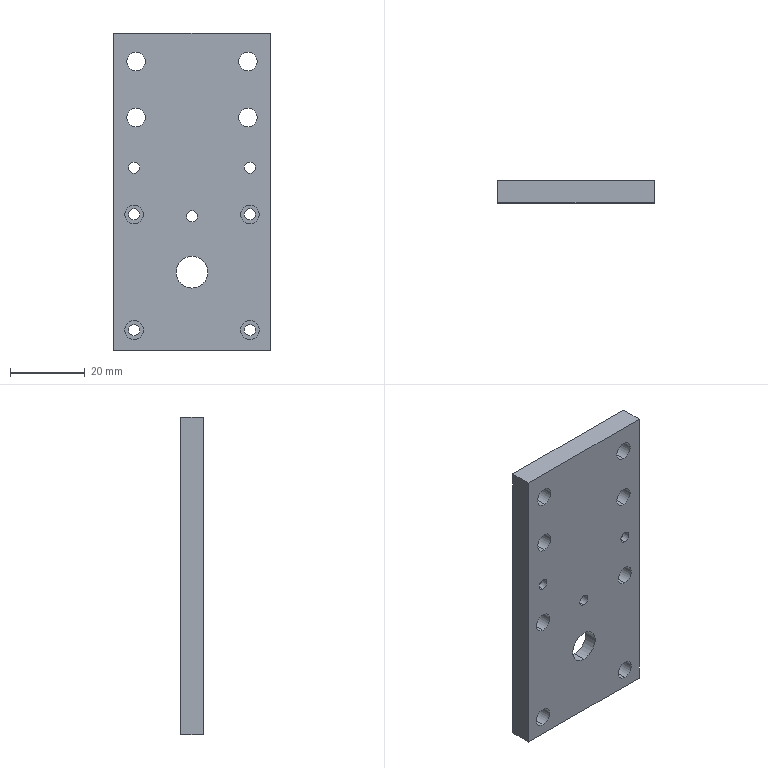Part | SolidWorks | features ICE 5, Cut 3, FlatPattern 1, SMBaseFlange 1, SheetMetal 1 | 1 solid | 51 faces | box 42 x 6 x 85 mm | volume 19158 mm3 | cylinder 38 | plane 13 | commonest cylinder face diameters 5 x20 3 x14 8.5 x2 22.5 x2
STEP:
#1=CARTESIAN_POINT('',(-15.,-6.,32.5));
#2=VERTEX_POINT('',#1);
#3=CARTESIAN_POINT('',(-15.,-6.,37.5));
#4=VERTEX_POINT('',#3);
#5=CARTESIAN_POINT('',(-15.,-6.,35.));
#6=DIRECTION('',(0.,1.,0.));
#7=DIRECTION('',(0.,0.,1.));
#8=AXIS2_PLACEMENT_3D('',#5,#6,#7);
#9=CIRCLE('',#8,2.5);
#10=EDGE_CURVE('',#2,#4,#9,.T.);
#11=ORIENTED_EDGE('',*,*,#10,.F.);
#12=CARTESIAN_POINT('',(-15.,0.,32.5));
#13=VERTEX_POINT('',#12);
#14=CARTESIAN_POINT('',(-15.,-6.,32.5));
#15=DIRECTION('',(0.,1.,0.));
#16=VECTOR('',#15,1000.);
#17=LINE('',#14,#16);
#18=EDGE_CURVE('',#2,#13,#17,.T.);
#19=ORIENTED_EDGE('',*,*,#18,.T.);
#20=CARTESIAN_POINT('',(-15.,0.,37.5));
#21=VERTEX_POINT('',#20);
#22=CARTESIAN_POINT('',(-15.,0.,35.));
#23=DIRECTION('',(0.,1.,0.));
#24=DIRECTION('',(0.,0.,1.));
#25=AXIS2_PLACEMENT_3D('',#22,#23,#24);
#26=CIRCLE('',#25,2.5);
#27=EDGE_CURVE('',#13,#21,#26,.T.);
#28=ORIENTED_EDGE('',*,*,#27,.T.);
#29=CARTESIAN_POINT('',(-15.,-6.,37.5));
#30=DIRECTION('',(0.,1.,0.));
#31=VECTOR('',#30,1000.);
#32=LINE('',#29,#31);
#33=EDGE_CURVE('',#4,#21,#32,.T.);
#34=ORIENTED_EDGE('',*,*,#33,.F.);
#35=EDGE_LOOP('',(#11,#19,#28,#34));
#36=FACE_OUTER_BOUND('',#35,.T.);
#37=CARTESIAN_POINT('',(-15.,-6.,35.));
#38=DIRECTION('',(0.,1.,0.));
#39=DIRECTION('',(0.,0.,1.));
#40=AXIS2_PLACEMENT_3D('',#37,#38,#39);
#41=CYLINDRICAL_SURFACE('',#40,2.5);
#42=ADVANCED_FACE('',(#36),#41,.F.);
#43=CARTESIAN_POINT('',(15.,-6.,32.5));
#44=VERTEX_POINT('',#43);
#45=CARTESIAN_POINT('',(15.,-6.,37.5));
#46=VERTEX_POINT('',#45);
#47=CARTESIAN_POINT('',(15.,-6.,35.));
#48=DIRECTION('',(0.,1.,0.));
#49=DIRECTION('',(0.,0.,1.));
#50=AXIS2_PLACEMENT_3D('',#47,#48,#49);
#51=CIRCLE('',#50,2.5);
#52=EDGE_CURVE('',#44,#46,#51,.T.);
#53=ORIENTED_EDGE('',*,*,#52,.F.);
#54=CARTESIAN_POINT('',(15.,0.,32.5));
#55=VERTEX_POINT('',#54);
#56=CARTESIAN_POINT('',(15.,-6.,32.5));
#57=DIRECTION('',(0.,1.,0.));
#58=VECTOR('',#57,1000.);
#59=LINE('',#56,#58);
#60=EDGE_CURVE('',#44,#55,#59,.T.);
#61=ORIENTED_EDGE('',*,*,#60,.T.);
#62=CARTESIAN_POINT('',(15.,0.,37.5));
#63=VERTEX_POINT('',#62);
#64=CARTESIAN_POINT('',(15.,0.,35.));
#65=DIRECTION('',(0.,1.,0.));
#66=DIRECTION('',(0.,0.,1.));
#67=AXIS2_PLACEMENT_3D('',#64,#65,#66);
#68=CIRCLE('',#67,2.5);
#69=EDGE_CURVE('',#55,#63,#68,.T.);
#70=ORIENTED_EDGE('',*,*,#69,.T.);
#71=CARTESIAN_POINT('',(15.,-6.,37.5));
#72=DIRECTION('',(0.,1.,0.));
#73=VECTOR('',#72,1000.);
#74=LINE('',#71,#73);
#75=EDGE_CURVE('',#46,#63,#74,.T.);
#76=ORIENTED_EDGE('',*,*,#75,.F.);
#77=EDGE_LOOP('',(#53,#61,#70,#76));
#78=FACE_OUTER_BOUND('',#77,.T.);
#79=CARTESIAN_POINT('',(15.,-6.,35.));
#80=DIRECTION('',(0.,1.,0.));
#81=DIRECTION('',(0.,0.,1.));
#82=AXIS2_PLACEMENT_3D('',#79,#80,#81);
#83=CYLINDRICAL_SURFACE('',#82,2.5);
#84=ADVANCED_FACE('',(#78),#83,.F.);
#85=CARTESIAN_POINT('',(15.,-6.,17.5));
#86=VERTEX_POINT('',#85);
#87=CARTESIAN_POINT('',(15.,-6.,22.5));
#88=VERTEX_POINT('',#87);
#89=CARTESIAN_POINT('',(15.,-6.,20.));
#90=DIRECTION('',(0.,1.,0.));
#91=DIRECTION('',(0.,0.,1.));
#92=AXIS2_PLACEMENT_3D('',#89,#90,#91);
#93=CIRCLE('',#92,2.5);
#94=EDGE_CURVE('',#86,#88,#93,.T.);
#95=ORIENTED_EDGE('',*,*,#94,.F.);
#96=CARTESIAN_POINT('',(15.,0.,17.5));
#97=VERTEX_POINT('',#96);
#98=CARTESIAN_POINT('',(15.,-6.,17.5));
#99=DIRECTION('',(0.,1.,0.));
#100=VECTOR('',#99,1000.);
#101=LINE('',#98,#100);
#102=EDGE_CURVE('',#86,#97,#101,.T.);
#103=ORIENTED_EDGE('',*,*,#102,.T.);
#104=CARTESIAN_POINT('',(15.,0.,22.5));
#105=VERTEX_POINT('',#104);
#106=CARTESIAN_POINT('',(15.,0.,20.));
#107=DIRECTION('',(0.,1.,0.));
#108=DIRECTION('',(0.,0.,1.));
#109=AXIS2_PLACEMENT_3D('',#106,#107,#108);
#110=CIRCLE('',#109,2.5);
#111=EDGE_CURVE('',#97,#105,#110,.T.);
#112=ORIENTED_EDGE('',*,*,#111,.T.);
#113=CARTESIAN_POINT('',(15.,-6.,22.5));
#114=DIRECTION('',(0.,1.,0.));
#115=VECTOR('',#114,1000.);
#116=LINE('',#113,#115);
#117=EDGE_CURVE('',#88,#105,#116,.T.);
#118=ORIENTED_EDGE('',*,*,#117,.F.);
#119=EDGE_LOOP('',(#95,#103,#112,#118));
#120=FACE_OUTER_BOUND('',#119,.T.);
#121=CARTESIAN_POINT('',(15.,-6.,20.));
#122=DIRECTION('',(0.,1.,0.));
#123=DIRECTION('',(0.,0.,1.));
#124=AXIS2_PLACEMENT_3D('',#121,#122,#123);
#125=CYLINDRICAL_SURFACE('',#124,2.5);
#126=ADVANCED_FACE('',(#120),#125,.F.);
#127=CARTESIAN_POINT('',(-15.,-6.,17.5));
#128=VERTEX_POINT('',#127);
#129=CARTESIAN_POINT('',(-15.,-6.,22.5));
#130=VERTEX_POINT('',#129);
#131=CARTESIAN_POINT('',(-15.,-6.,20.));
#132=DIRECTION('',(0.,1.,0.));
#133=DIRECTION('',(0.,0.,1.));
#134=AXIS2_PLACEMENT_3D('',#131,#132,#133);
#135=CIRCLE('',#134,2.5);
#136=EDGE_CURVE('',#128,#130,#135,.T.);
#137=ORIENTED_EDGE('',*,*,#136,.F.);
#138=CARTESIAN_POINT('',(-15.,0.,17.5));
#139=VERTEX_POINT('',#138);
#140=CARTESIAN_POINT('',(-15.,-6.,17.5));
#141=DIRECTION('',(0.,1.,0.));
#142=VECTOR('',#141,1000.);
#143=LINE('',#140,#142);
#144=EDGE_CURVE('',#128,#139,#143,.T.);
#145=ORIENTED_EDGE('',*,*,#144,.T.);
#146=CARTESIAN_POINT('',(-15.,0.,22.5));
#147=VERTEX_POINT('',#146);
#148=CARTESIAN_POINT('',(-15.,0.,20.));
#149=DIRECTION('',(0.,1.,0.));
#150=DIRECTION('',(0.,0.,1.));
#151=AXIS2_PLACEMENT_3D('',#148,#149,#150);
#152=CIRCLE('',#151,2.5);
#153=EDGE_CURVE('',#139,#147,#152,.T.);
#154=ORIENTED_EDGE('',*,*,#153,.T.);
#155=CARTESIAN_POINT('',(-15.,-6.,22.5));
#156=DIRECTION('',(0.,1.,0.));
#157=VECTOR('',#156,1000.);
#158=LINE('',#155,#157);
#159=EDGE_CURVE('',#130,#147,#158,.T.);
#160=ORIENTED_EDGE('',*,*,#159,.F.);
#161=EDGE_LOOP('',(#137,#145,#154,#160));
#162=FACE_OUTER_BOUND('',#161,.T.);
#163=CARTESIAN_POINT('',(-15.,-6.,20.));
#164=DIRECTION('',(0.,1.,0.));
#165=DIRECTION('',(0.,0.,1.));
#166=AXIS2_PLACEMENT_3D('',#163,#164,#165);
#167=CYLINDRICAL_SURFACE('',#166,2.5);
#168=ADVANCED_FACE('',(#162),#167,.F.);
#169=CARTESIAN_POINT('',(15.5,-4.,4.));
#170=VERTEX_POINT('',#169);
#171=CARTESIAN_POINT('',(15.5,-4.,9.));
#172=VERTEX_POINT('',#171);
#173=CARTESIAN_POINT('',(15.5,-4.,6.5));
#174=DIRECTION('',(0.,1.,0.));
#175=DIRECTION('',(0.,0.,1.));
#176=AXIS2_PLACEMENT_3D('',#173,#174,#175);
#177=CIRCLE('',#176,2.5);
#178=EDGE_CURVE('',#170,#172,#177,.T.);
#179=ORIENTED_EDGE('',*,*,#178,.F.);
#180=CARTESIAN_POINT('',(15.5,0.,4.));
#181=VERTEX_POINT('',#180);
#182=CARTESIAN_POINT('',(15.5,-4.,4.));
#183=DIRECTION('',(0.,1.,0.));
#184=VECTOR('',#183,1000.);
#185=LINE('',#182,#184);
#186=EDGE_CURVE('',#170,#181,#185,.T.);
#187=ORIENTED_EDGE('',*,*,#186,.T.);
#188=CARTESIAN_POINT('',(15.5,0.,9.));
#189=VERTEX_POINT('',#188);
#190=CARTESIAN_POINT('',(15.5,0.,6.5));
#191=DIRECTION('',(0.,1.,0.));
#192=DIRECTION('',(0.,0.,1.));
#193=AXIS2_PLACEMENT_3D('',#190,#191,#192);
#194=CIRCLE('',#193,2.5);
#195=EDGE_CURVE('',#181,#189,#194,.T.);
#196=ORIENTED_EDGE('',*,*,#195,.T.);
#197=CARTESIAN_POINT('',(15.5,-4.,9.));
#198=DIRECTION('',(0.,1.,0.));
#199=VECTOR('',#198,1000.);
#200=LINE('',#197,#199);
#201=EDGE_CURVE('',#172,#189,#200,.T.);
#202=ORIENTED_EDGE('',*,*,#201,.F.);
#203=EDGE_LOOP('',(#179,#187,#196,#202));
#204=FACE_OUTER_BOUND('',#203,.T.);
#205=CARTESIAN_POINT('',(15.5,-4.,6.5));
#206=DIRECTION('',(0.,1.,0.));
#207=DIRECTION('',(0.,0.,1.));
#208=AXIS2_PLACEMENT_3D('',#205,#206,#207);
#209=CYLINDRICAL_SURFACE('',#208,2.5);
#210=ADVANCED_FACE('',(#204),#209,.F.);
#211=CARTESIAN_POINT('',(-15.5,-4.,4.));
#212=VERTEX_POINT('',#211);
#213=CARTESIAN_POINT('',(-15.5,-4.,9.));
#214=VERTEX_POINT('',#213);
#215=CARTESIAN_POINT('',(-15.5,-4.,6.5));
#216=DIRECTION('',(0.,1.,0.));
#217=DIRECTION('',(0.,0.,1.));
#218=AXIS2_PLACEMENT_3D('',#215,#216,#217);
#219=CIRCLE('',#218,2.5);
#220=EDGE_CURVE('',#212,#214,#219,.T.);
#221=ORIENTED_EDGE('',*,*,#220,.F.);
#222=CARTESIAN_POINT('',(-15.5,0.,4.));
#223=VERTEX_POINT('',#222);
#224=CARTESIAN_POINT('',(-15.5,-4.,4.));
#225=DIRECTION('',(0.,1.,0.));
#226=VECTOR('',#225,1000.);
#227=LINE('',#224,#226);
#228=EDGE_CURVE('',#212,#223,#227,.T.);
#229=ORIENTED_EDGE('',*,*,#228,.T.);
#230=CARTESIAN_POINT('',(-15.5,0.,9.));
#231=VERTEX_POINT('',#230);
#232=CARTESIAN_POINT('',(-15.5,0.,6.5));
#233=DIRECTION('',(0.,1.,0.));
#234=DIRECTION('',(0.,0.,1.));
#235=AXIS2_PLACEMENT_3D('',#232,#233,#234);
#236=CIRCLE('',#235,2.5);
#237=EDGE_CURVE('',#223,#231,#236,.T.);
#238=ORIENTED_EDGE('',*,*,#237,.T.);
#239=CARTESIAN_POINT('',(-15.5,-4.,9.));
#240=DIRECTION('',(0.,1.,0.));
#241=VECTOR('',#240,1000.);
#242=LINE('',#239,#241);
#243=EDGE_CURVE('',#214,#231,#242,.T.);
#244=ORIENTED_EDGE('',*,*,#243,.F.);
#245=EDGE_LOOP('',(#221,#229,#238,#244));
#246=FACE_OUTER_BOUND('',#245,.T.);
#247=CARTESIAN_POINT('',(-15.5,-4.,6.5));
#248=DIRECTION('',(0.,1.,0.));
#249=DIRECTION('',(0.,0.,1.));
#250=AXIS2_PLACEMENT_3D('',#247,#248,#249);
#251=CYLINDRICAL_SURFACE('',#250,2.5);
#252=ADVANCED_FACE('',(#246),#251,.F.);
#253=CARTESIAN_POINT('',(15.5,-2.,-3.5));
#254=VERTEX_POINT('',#253);
#255=CARTESIAN_POINT('',(15.5,-2.,-8.5));
#256=VERTEX_POINT('',#255);
#257=CARTESIAN_POINT('',(15.5,-2.,-6.));
#258=DIRECTION('',(0.,-1.,0.));
#259=DIRECTION('',(0.,0.,-1.));
#260=AXIS2_PLACEMENT_3D('',#257,#258,#259);
#261=CIRCLE('',#260,2.5);
#262=EDGE_CURVE('',#254,#256,#261,.T.);
#263=ORIENTED_EDGE('',*,*,#262,.F.);
#264=CARTESIAN_POINT('',(15.5,-6.,-3.5));
#265=VERTEX_POINT('',#264);
#266=CARTESIAN_POINT('',(15.5,-2.,-3.5));
#267=DIRECTION('',(0.,-1.,0.));
#268=VECTOR('',#267,1000.);
#269=LINE('',#266,#268);
#270=EDGE_CURVE('',#254,#265,#269,.T.);
#271=ORIENTED_EDGE('',*,*,#270,.T.);
#272=CARTESIAN_POINT('',(15.5,-6.,-8.5));
#273=VERTEX_POINT('',#272);
#274=CARTESIAN_POINT('',(15.5,-6.,-6.));
#275=DIRECTION('',(0.,-1.,0.));
#276=DIRECTION('',(0.,0.,-1.));
#277=AXIS2_PLACEMENT_3D('',#274,#275,#276);
#278=CIRCLE('',#277,2.5);
#279=EDGE_CURVE('',#265,#273,#278,.T.);
#280=ORIENTED_EDGE('',*,*,#279,.T.);
#281=CARTESIAN_POINT('',(15.5,-2.,-8.5));
#282=DIRECTION('',(0.,-1.,0.));
#283=VECTOR('',#282,1000.);
#284=LINE('',#281,#283);
#285=EDGE_CURVE('',#256,#273,#284,.T.);
#286=ORIENTED_EDGE('',*,*,#285,.F.);
#287=EDGE_LOOP('',(#263,#271,#280,#286));
#288=FACE_OUTER_BOUND('',#287,.T.);
#289=CARTESIAN_POINT('',(15.5,-2.,-6.));
#290=DIRECTION('',(0.,-1.,0.));
#291=DIRECTION('',(0.,0.,-1.));
#292=AXIS2_PLACEMENT_3D('',#289,#290,#291);
#293=CYLINDRICAL_SURFACE('',#292,2.5);
#294=ADVANCED_FACE('',(#288),#293,.F.);
#295=CARTESIAN_POINT('',(-15.5,-2.,-3.5));
#296=VERTEX_POINT('',#295);
#297=CARTESIAN_POINT('',(-15.5,-2.,-8.5));
#298=VERTEX_POINT('',#297);
#299=CARTESIAN_POINT('',(-15.5,-2.,-6.));
#300=DIRECTION('',(0.,-1.,0.));
#301=DIRECTION('',(0.,0.,-1.));
#302=AXIS2_PLACEMENT_3D('',#299,#300,#301);
#303=CIRCLE('',#302,2.5);
#304=EDGE_CURVE('',#296,#298,#303,.T.);
#305=ORIENTED_EDGE('',*,*,#304,.F.);
#306=CARTESIAN_POINT('',(-15.5,-6.,-3.5));
#307=VERTEX_POINT('',#306);
#308=CARTESIAN_POINT('',(-15.5,-2.,-3.5));
#309=DIRECTION('',(0.,-1.,0.));
#310=VECTOR('',#309,1000.);
#311=LINE('',#308,#310);
#312=EDGE_CURVE('',#296,#307,#311,.T.);
#313=ORIENTED_EDGE('',*,*,#312,.T.);
#314=CARTESIAN_POINT('',(-15.5,-6.,-8.5));
#315=VERTEX_POINT('',#314);
#316=CARTESIAN_POINT('',(-15.5,-6.,-6.));
#317=DIRECTION('',(0.,-1.,0.));
#318=DIRECTION('',(0.,0.,-1.));
#319=AXIS2_PLACEMENT_3D('',#316,#317,#318);
#320=CIRCLE('',#319,2.5);
#321=EDGE_CURVE('',#307,#315,#320,.T.);
#322=ORIENTED_EDGE('',*,*,#321,.T.);
#323=CARTESIAN_POINT('',(-15.5,-2.,-8.5));
#324=DIRECTION('',(0.,-1.,0.));
#325=VECTOR('',#324,1000.);
#326=LINE('',#323,#325);
#327=EDGE_CURVE('',#298,#315,#326,.T.);
#328=ORIENTED_EDGE('',*,*,#327,.F.);
#329=EDGE_LOOP('',(#305,#313,#322,#328));
#330=FACE_OUTER_BOUND('',#329,.T.);
#331=CARTESIAN_POINT('',(-15.5,-2.,-6.));
#332=DIRECTION('',(0.,-1.,0.));
#333=DIRECTION('',(0.,0.,-1.));
#334=AXIS2_PLACEMENT_3D('',#331,#332,#333);
#335=CYLINDRICAL_SURFACE('',#334,2.5);
#336=ADVANCED_FACE('',(#330),#335,.F.);
#337=CARTESIAN_POINT('',(-15.5,-6.,-39.5));
#338=VERTEX_POINT('',#337);
#339=CARTESIAN_POINT('',(-15.5,-6.,-34.5));
#340=VERTEX_POINT('',#339);
#341=CARTESIAN_POINT('',(-15.5,-6.,-37.));
#342=DIRECTION('',(0.,1.,0.));
#343=DIRECTION('',(0.,0.,1.));
#344=AXIS2_PLACEMENT_3D('',#341,#342,#343);
#345=CIRCLE('',#344,2.5);
#346=EDGE_CURVE('',#338,#340,#345,.T.);
#347=ORIENTED_EDGE('',*,*,#346,.F.);
#348=CARTESIAN_POINT('',(-15.5,-2.,-39.5));
#349=VERTEX_POINT('',#348);
#350=CARTESIAN_POINT('',(-15.5,-6.,-39.5));
#351=DIRECTION('',(0.,1.,0.));
#352=VECTOR('',#351,1000.);
#353=LINE('',#350,#352);
#354=EDGE_CURVE('',#338,#349,#353,.T.);
#355=ORIENTED_EDGE('',*,*,#354,.T.);
#356=CARTESIAN_POINT('',(-15.5,-2.,-34.5));
#357=VERTEX_POINT('',#356);
#358=CARTESIAN_POINT('',(-15.5,-2.,-37.));
#359=DIRECTION('',(0.,1.,0.));
#360=DIRECTION('',(0.,0.,1.));
#361=AXIS2_PLACEMENT_3D('',#358,#359,#360);
#362=CIRCLE('',#361,2.5);
#363=EDGE_CURVE('',#349,#357,#362,.T.);
#364=ORIENTED_EDGE('',*,*,#363,.T.);
#365=CARTESIAN_POINT('',(-15.5,-6.,-34.5));
#366=DIRECTION('',(0.,1.,0.));
#367=VECTOR('',#366,1000.);
#368=LINE('',#365,#367);
#369=EDGE_CURVE('',#340,#357,#368,.T.);
#370=ORIENTED_EDGE('',*,*,#369,.F.);
#371=EDGE_LOOP('',(#347,#355,#364,#370));
#372=FACE_OUTER_BOUND('',#371,.T.);
#373=CARTESIAN_POINT('',(-15.5,-6.,-37.));
#374=DIRECTION('',(0.,1.,0.));
#375=DIRECTION('',(0.,0.,1.));
#376=AXIS2_PLACEMENT_3D('',#373,#374,#375);
#377=CYLINDRICAL_SURFACE('',#376,2.5);
#378=ADVANCED_FACE('',(#372),#377,.F.);
#379=CARTESIAN_POINT('',(15.5,-6.,-39.5));
#380=VERTEX_POINT('',#379);
#381=CARTESIAN_POINT('',(15.5,-6.,-34.5));
#382=VERTEX_POINT('',#381);
#383=CARTESIAN_POINT('',(15.5,-6.,-37.));
#384=DIRECTION('',(0.,1.,0.));
#385=DIRECTION('',(0.,0.,1.));
#386=AXIS2_PLACEMENT_3D('',#383,#384,#385);
#387=CIRCLE('',#386,2.5);
#388=EDGE_CURVE('',#380,#382,#387,.T.);
#389=ORIENTED_EDGE('',*,*,#388,.F.);
#390=CARTESIAN_POINT('',(15.5,-2.,-39.5));
#391=VERTEX_POINT('',#390);
#392=CARTESIAN_POINT('',(15.5,-6.,-39.5));
#393=DIRECTION('',(0.,1.,0.));
#394=VECTOR('',#393,1000.);
#395=LINE('',#392,#394);
#396=EDGE_CURVE('',#380,#391,#395,.T.);
#397=ORIENTED_EDGE('',*,*,#396,.T.);
#398=CARTESIAN_POINT('',(15.5,-2.,-34.5));
#399=VERTEX_POINT('',#398);
#400=CARTESIAN_POINT('',(15.5,-2.,-37.));
#401=DIRECTION('',(0.,1.,0.));
#402=DIRECTION('',(0.,0.,1.));
#403=AXIS2_PLACEMENT_3D('',#400,#401,#402);
#404=CIRCLE('',#403,2.5);
#405=EDGE_CURVE('',#391,#399,#404,.T.);
#406=ORIENTED_EDGE('',*,*,#405,.T.);
#407=CARTESIAN_POINT('',(15.5,-6.,-34.5));
#408=DIRECTION('',(0.,1.,0.));
#409=VECTOR('',#408,1000.);
#410=LINE('',#407,#409);
#411=EDGE_CURVE('',#382,#399,#410,.T.);
#412=ORIENTED_EDGE('',*,*,#411,.F.);
#413=EDGE_LOOP('',(#389,#397,#406,#412));
#414=FACE_OUTER_BOUND('',#413,.T.);
#415=CARTESIAN_POINT('',(15.5,-6.,-37.));
#416=DIRECTION('',(0.,1.,0.));
#417=DIRECTION('',(0.,0.,1.));
#418=AXIS2_PLACEMENT_3D('',#415,#416,#417);
#419=CYLINDRICAL_SURFACE('',#418,2.5);
#420=ADVANCED_FACE('',(#414),#419,.F.);
#421=CARTESIAN_POINT('',(15.5,-2.,-35.5));
#422=VERTEX_POINT('',#421);
#423=CARTESIAN_POINT('',(15.5,-2.,-38.5));
#424=VERTEX_POINT('',#423);
#425=CARTESIAN_POINT('',(15.5,-2.,-37.));
#426=DIRECTION('',(0.,-1.,0.));
#427=DIRECTION('',(0.,0.,1.));
#428=AXIS2_PLACEMENT_3D('',#425,#426,#427);
#429=CIRCLE('',#428,1.5);
#430=EDGE_CURVE('',#422,#424,#429,.T.);
#431=ORIENTED_EDGE('',*,*,#430,.T.);
#432=CARTESIAN_POINT('',(15.5,0.,-38.5));
#433=VERTEX_POINT('',#432);
#434=CARTESIAN_POINT('',(15.5,-6.,-38.5));
#435=DIRECTION('',(0.,1.,0.));
#436=VECTOR('',#435,1000.);
#437=LINE('',#434,#436);
#438=EDGE_CURVE('',#424,#433,#437,.T.);
#439=ORIENTED_EDGE('',*,*,#438,.T.);
#440=CARTESIAN_POINT('',(15.5,0.,-35.5));
#441=VERTEX_POINT('',#440);
#442=CARTESIAN_POINT('',(15.5,0.,-37.));
#443=DIRECTION('',(0.,1.,0.));
#444=DIRECTION('',(0.,0.,1.));
#445=AXIS2_PLACEMENT_3D('',#442,#443,#444);
#446=CIRCLE('',#445,1.5);
#447=EDGE_CURVE('',#433,#441,#446,.T.);
#448=ORIENTED_EDGE('',*,*,#447,.T.);
#449=CARTESIAN_POINT('',(15.5,-6.,-35.5));
#450=DIRECTION('',(0.,1.,0.));
#451=VECTOR('',#450,1000.);
#452=LINE('',#449,#451);
#453=EDGE_CURVE('',#422,#441,#452,.T.);
#454=ORIENTED_EDGE('',*,*,#453,.F.);
#455=EDGE_LOOP('',(#431,#439,#448,#454));
#456=FACE_OUTER_BOUND('',#455,.T.);
#457=CARTESIAN_POINT('',(15.5,-6.,-37.));
#458=DIRECTION('',(0.,1.,0.));
#459=DIRECTION('',(0.,0.,1.));
#460=AXIS2_PLACEMENT_3D('',#457,#458,#459);
#461=CYLINDRICAL_SURFACE('',#460,1.5);
#462=ADVANCED_FACE('',(#456),#461,.F.);
#463=CARTESIAN_POINT('',(-15.5,-2.,-35.5));
#464=VERTEX_POINT('',#463);
#465=CARTESIAN_POINT('',(-15.5,-2.,-38.5));
#466=VERTEX_POINT('',#465);
#467=CARTESIAN_POINT('',(-15.5,-2.,-37.));
#468=DIRECTION('',(0.,-1.,0.));
#469=DIRECTION('',(0.,0.,1.));
#470=AXIS2_PLACEMENT_3D('',#467,#468,#469);
#471=CIRCLE('',#470,1.5);
#472=EDGE_CURVE('',#464,#466,#471,.T.);
#473=ORIENTED_EDGE('',*,*,#472,.T.);
#474=CARTESIAN_POINT('',(-15.5,0.,-38.5));
#475=VERTEX_POINT('',#474);
#476=CARTESIAN_POINT('',(-15.5,-6.,-38.5));
#477=DIRECTION('',(0.,1.,0.));
#478=VECTOR('',#477,1000.);
#479=LINE('',#476,#478);
#480=EDGE_CURVE('',#466,#475,#479,.T.);
#481=ORIENTED_EDGE('',*,*,#480,.T.);
#482=CARTESIAN_POINT('',(-15.5,0.,-35.5));
#483=VERTEX_POINT('',#482);
#484=CARTESIAN_POINT('',(-15.5,0.,-37.));
#485=DIRECTION('',(0.,1.,0.));
#486=DIRECTION('',(0.,0.,1.));
#487=AXIS2_PLACEMENT_3D('',#484,#485,#486);
#488=CIRCLE('',#487,1.5);
#489=EDGE_CURVE('',#475,#483,#488,.T.);
#490=ORIENTED_EDGE('',*,*,#489,.T.);
#491=CARTESIAN_POINT('',(-15.5,-6.,-35.5));
#492=DIRECTION('',(0.,1.,0.));
#493=VECTOR('',#492,1000.);
#494=LINE('',#491,#493);
#495=EDGE_CURVE('',#464,#483,#494,.T.);
#496=ORIENTED_EDGE('',*,*,#495,.F.);
#497=EDGE_LOOP('',(#473,#481,#490,#496));
#498=FACE_OUTER_BOUND('',#497,.T.);
#499=CARTESIAN_POINT('',(-15.5,-6.,-37.));
#500=DIRECTION('',(0.,1.,0.));
#501=DIRECTION('',(0.,0.,1.));
#502=AXIS2_PLACEMENT_3D('',#499,#500,#501);
#503=CYLINDRICAL_SURFACE('',#502,1.5);
#504=ADVANCED_FACE('',(#498),#503,.F.);
#505=CARTESIAN_POINT('',(0.,-2.5,-32.75));
#506=VERTEX_POINT('',#505);
#507=CARTESIAN_POINT('',(0.,-2.5,-10.25));
#508=VERTEX_POINT('',#507);
#509=CARTESIAN_POINT('',(0.,-2.5,-21.5));
#510=DIRECTION('',(0.,1.,0.));
#511=DIRECTION('',(0.,0.,1.));
#512=AXIS2_PLACEMENT_3D('',#509,#510,#511);
#513=CIRCLE('',#512,11.25);
#514=EDGE_CURVE('',#506,#508,#513,.T.);
#515=ORIENTED_EDGE('',*,*,#514,.F.);
#516=CARTESIAN_POINT('',(0.,0.,-32.75));
#517=VERTEX_POINT('',#516);
#518=CARTESIAN_POINT('',(0.,-2.5,-32.75));
#519=DIRECTION('',(0.,1.,0.));
#520=VECTOR('',#519,1000.);
#521=LINE('',#518,#520);
#522=EDGE_CURVE('',#506,#517,#521,.T.);
#523=ORIENTED_EDGE('',*,*,#522,.T.);
#524=CARTESIAN_POINT('',(0.,0.,-10.25));
#525=VERTEX_POINT('',#524);
#526=CARTESIAN_POINT('',(0.,0.,-21.5));
#527=DIRECTION('',(0.,1.,0.));
#528=DIRECTION('',(0.,0.,1.));
#529=AXIS2_PLACEMENT_3D('',#526,#527,#528);
#530=CIRCLE('',#529,11.25);
#531=EDGE_CURVE('',#517,#525,#530,.T.);
#532=ORIENTED_EDGE('',*,*,#531,.T.);
#533=CARTESIAN_POINT('',(0.,-2.5,-10.25));
#534=DIRECTION('',(0.,1.,0.));
#535=VECTOR('',#534,1000.);
#536=LINE('',#533,#535);
#537=EDGE_CURVE('',#508,#525,#536,.T.);
#538=ORIENTED_EDGE('',*,*,#537,.F.);
#539=EDGE_LOOP('',(#515,#523,#532,#538));
#540=FACE_OUTER_BOUND('',#539,.T.);
#541=CARTESIAN_POINT('',(0.,-2.5,-21.5));
#542=DIRECTION('',(0.,1.,0.));
#543=DIRECTION('',(0.,0.,1.));
#544=AXIS2_PLACEMENT_3D('',#541,#542,#543);
#545=CYLINDRICAL_SURFACE('',#544,11.25);
#546=ADVANCED_FACE('',(#540),#545,.F.);
#547=CARTESIAN_POINT('',(0.,-6.,-5.));
#548=VERTEX_POINT('',#547);
#549=CARTESIAN_POINT('',(0.,-6.,-8.));
#550=VERTEX_POINT('',#549);
#551=CARTESIAN_POINT('',(0.,-6.,-6.5));
#552=DIRECTION('',(0.,-1.,0.));
#553=DIRECTION('',(0.,0.,1.));
#554=AXIS2_PLACEMENT_3D('',#551,#552,#553);
#555=CIRCLE('',#554,1.5);
#556=EDGE_CURVE('',#548,#550,#555,.T.);
#557=ORIENTED_EDGE('',*,*,#556,.T.);
#558=CARTESIAN_POINT('',(0.,0.,-8.));
#559=VERTEX_POINT('',#558);
#560=CARTESIAN_POINT('',(0.,-6.001,-8.));
#561=DIRECTION('',(0.,1.,0.));
#562=VECTOR('',#561,1000.);
#563=LINE('',#560,#562);
#564=EDGE_CURVE('',#550,#559,#563,.T.);
#565=ORIENTED_EDGE('',*,*,#564,.T.);
#566=CARTESIAN_POINT('',(0.,0.,-5.));
#567=VERTEX_POINT('',#566);
#568=CARTESIAN_POINT('',(0.,0.,-6.5));
#569=DIRECTION('',(0.,1.,0.));
#570=DIRECTION('',(0.,0.,1.));
#571=AXIS2_PLACEMENT_3D('',#568,#569,#570);
#572=CIRCLE('',#571,1.5);
#573=EDGE_CURVE('',#559,#567,#572,.T.);
#574=ORIENTED_EDGE('',*,*,#573,.T.);
#575=CARTESIAN_POINT('',(0.,-6.001,-5.));
#576=DIRECTION('',(0.,1.,0.));
#577=VECTOR('',#576,1000.);
#578=LINE('',#575,#577);
#579=EDGE_CURVE('',#548,#567,#578,.T.);
#580=ORIENTED_EDGE('',*,*,#579,.F.);
#581=EDGE_LOOP('',(#557,#565,#574,#580));
#582=FACE_OUTER_BOUND('',#581,.T.);
#583=CARTESIAN_POINT('',(0.,-6.001,-6.5));
#584=DIRECTION('',(0.,1.,0.));
#585=DIRECTION('',(0.,0.,1.));
#586=AXIS2_PLACEMENT_3D('',#583,#584,#585);
#587=CYLINDRICAL_SURFACE('',#586,1.5);
#588=ADVANCED_FACE('',(#582),#587,.F.);
#589=CARTESIAN_POINT('',(0.,-6.,-17.25));
#590=VERTEX_POINT('',#589);
#591=CARTESIAN_POINT('',(0.,-6.,-25.75));
#592=VERTEX_POINT('',#591);
#593=CARTESIAN_POINT('',(0.,-6.,-21.5));
#594=DIRECTION('',(0.,-1.,0.));
#595=DIRECTION('',(0.,0.,1.));
#596=AXIS2_PLACEMENT_3D('',#593,#594,#595);
#597=CIRCLE('',#596,4.25);
#598=EDGE_CURVE('',#590,#592,#597,.T.);
#599=ORIENTED_EDGE('',*,*,#598,.T.);
#600=CARTESIAN_POINT('',(0.,-2.5,-25.75));
#601=VERTEX_POINT('',#600);
#602=CARTESIAN_POINT('',(0.,-6.001,-25.75));
#603=DIRECTION('',(0.,1.,0.));
#604=VECTOR('',#603,1000.);
#605=LINE('',#602,#604);
#606=EDGE_CURVE('',#592,#601,#605,.T.);
#607=ORIENTED_EDGE('',*,*,#606,.T.);
#608=CARTESIAN_POINT('',(0.,-2.5,-17.25));
#609=VERTEX_POINT('',#608);
#610=CARTESIAN_POINT('',(0.,-2.5,-21.5));
#611=DIRECTION('',(0.,-1.,0.));
#612=DIRECTION('',(0.,0.,1.));
#613=AXIS2_PLACEMENT_3D('',#610,#611,#612);
#614=CIRCLE('',#613,4.25);
#615=EDGE_CURVE('',#609,#601,#614,.T.);
#616=ORIENTED_EDGE('',*,*,#615,.F.);
#617=CARTESIAN_POINT('',(0.,-6.001,-17.25));
#618=DIRECTION('',(0.,1.,0.));
#619=VECTOR('',#618,1000.);
#620=LINE('',#617,#619);
#621=EDGE_CURVE('',#590,#609,#620,.T.);
#622=ORIENTED_EDGE('',*,*,#621,.F.);
#623=EDGE_LOOP('',(#599,#607,#616,#622));
#624=FACE_OUTER_BOUND('',#623,.T.);
#625=CARTESIAN_POINT('',(0.,-6.001,-21.5));
#626=DIRECTION('',(0.,1.,0.));
#627=DIRECTION('',(0.,0.,1.));
#628=AXIS2_PLACEMENT_3D('',#625,#626,#627);
#629=CYLINDRICAL_SURFACE('',#628,4.25);
#630=ADVANCED_FACE('',(#624),#629,.F.);
#631=CARTESIAN_POINT('',(-15.5,-2.,-7.5));
#632=VERTEX_POINT('',#631);
#633=CARTESIAN_POINT('',(-15.5,-2.,-4.5));
#634=VERTEX_POINT('',#633);
#635=CARTESIAN_POINT('',(-15.5,-2.,-6.));
#636=DIRECTION('',(0.,1.,0.));
#637=DIRECTION('',(0.,0.,-1.));
#638=AXIS2_PLACEMENT_3D('',#635,#636,#637);
#639=CIRCLE('',#638,1.5);
#640=EDGE_CURVE('',#632,#634,#639,.T.);
#641=ORIENTED_EDGE('',*,*,#640,.F.);
#642=CARTESIAN_POINT('',(-15.5,0.,-7.5));
#643=VERTEX_POINT('',#642);
#644=CARTESIAN_POINT('',(-15.5,-6.,-7.5));
#645=DIRECTION('',(0.,1.,0.));
#646=VECTOR('',#645,1000.);
#647=LINE('',#644,#646);
#648=EDGE_CURVE('',#632,#643,#647,.T.);
#649=ORIENTED_EDGE('',*,*,#648,.T.);
#650=CARTESIAN_POINT('',(-15.5,0.,-4.5));
#651=VERTEX_POINT('',#650);
#652=CARTESIAN_POINT('',(-15.5,0.,-6.));
#653=DIRECTION('',(0.,1.,0.));
#654=DIRECTION('',(0.,0.,1.));
#655=AXIS2_PLACEMENT_3D('',#652,#653,#654);
#656=CIRCLE('',#655,1.5);
#657=EDGE_CURVE('',#643,#651,#656,.T.);
#658=ORIENTED_EDGE('',*,*,#657,.T.);
#659=CARTESIAN_POINT('',(-15.5,-6.,-4.5));
#660=DIRECTION('',(0.,1.,0.));
#661=VECTOR('',#660,1000.);
#662=LINE('',#659,#661);
#663=EDGE_CURVE('',#634,#651,#662,.T.);
#664=ORIENTED_EDGE('',*,*,#663,.F.);
#665=EDGE_LOOP('',(#641,#649,#658,#664));
#666=FACE_OUTER_BOUND('',#665,.T.);
#667=CARTESIAN_POINT('',(-15.5,-6.,-6.));
#668=DIRECTION('',(0.,1.,0.));
#669=DIRECTION('',(0.,0.,1.));
#670=AXIS2_PLACEMENT_3D('',#667,#668,#669);
#671=CYLINDRICAL_SURFACE('',#670,1.5);
#672=ADVANCED_FACE('',(#666),#671,.F.);
#673=CARTESIAN_POINT('',(15.5,-2.,-7.5));
#674=VERTEX_POINT('',#673);
#675=CARTESIAN_POINT('',(15.5,-2.,-4.5));
#676=VERTEX_POINT('',#675);
#677=CARTESIAN_POINT('',(15.5,-2.,-6.));
#678=DIRECTION('',(0.,1.,0.));
#679=DIRECTION('',(0.,0.,-1.));
#680=AXIS2_PLACEMENT_3D('',#677,#678,#679);
#681=CIRCLE('',#680,1.5);
#682=EDGE_CURVE('',#674,#676,#681,.T.);
#683=ORIENTED_EDGE('',*,*,#682,.F.);
#684=CARTESIAN_POINT('',(15.5,0.,-7.5));
#685=VERTEX_POINT('',#684);
#686=CARTESIAN_POINT('',(15.5,-6.,-7.5));
#687=DIRECTION('',(0.,1.,0.));
#688=VECTOR('',#687,1000.);
#689=LINE('',#686,#688);
#690=EDGE_CURVE('',#674,#685,#689,.T.);
#691=ORIENTED_EDGE('',*,*,#690,.T.);
#692=CARTESIAN_POINT('',(15.5,0.,-4.5));
#693=VERTEX_POINT('',#692);
#694=CARTESIAN_POINT('',(15.5,0.,-6.));
#695=DIRECTION('',(0.,1.,0.));
#696=DIRECTION('',(0.,0.,1.));
#697=AXIS2_PLACEMENT_3D('',#694,#695,#696);
#698=CIRCLE('',#697,1.5);
#699=EDGE_CURVE('',#685,#693,#698,.T.);
#700=ORIENTED_EDGE('',*,*,#699,.T.);
#701=CARTESIAN_POINT('',(15.5,-6.,-4.5));
#702=DIRECTION('',(0.,1.,0.));
#703=VECTOR('',#702,1000.);
#704=LINE('',#701,#703);
#705=EDGE_CURVE('',#676,#693,#704,.T.);
#706=ORIENTED_EDGE('',*,*,#705,.F.);
#707=EDGE_LOOP('',(#683,#691,#700,#706));
#708=FACE_OUTER_BOUND('',#707,.T.);
#709=CARTESIAN_POINT('',(15.5,-6.,-6.));
#710=DIRECTION('',(0.,1.,0.));
#711=DIRECTION('',(0.,0.,1.));
#712=AXIS2_PLACEMENT_3D('',#709,#710,#711);
#713=CYLINDRICAL_SURFACE('',#712,1.5);
#714=ADVANCED_FACE('',(#708),#713,.F.);
#715=CARTESIAN_POINT('',(-15.5,-6.,5.));
#716=VERTEX_POINT('',#715);
#717=CARTESIAN_POINT('',(-15.5,-6.,8.));
#718=VERTEX_POINT('',#717);
#719=CARTESIAN_POINT('',(-15.5,-6.,6.5));
#720=DIRECTION('',(0.,1.,0.));
#721=DIRECTION('',(0.,0.,1.));
#722=AXIS2_PLACEMENT_3D('',#719,#720,#721);
#723=CIRCLE('',#722,1.5);
#724=EDGE_CURVE('',#716,#718,#723,.T.);
#725=ORIENTED_EDGE('',*,*,#724,.F.);
#726=CARTESIAN_POINT('',(-15.5,-4.,5.));
#727=VERTEX_POINT('',#726);
#728=CARTESIAN_POINT('',(-15.5,-6.,5.));
#729=DIRECTION('',(0.,1.,0.));
#730=VECTOR('',#729,1000.);
#731=LINE('',#728,#730);
#732=EDGE_CURVE('',#716,#727,#731,.T.);
#733=ORIENTED_EDGE('',*,*,#732,.T.);
#734=CARTESIAN_POINT('',(-15.5,-4.,8.));
#735=VERTEX_POINT('',#734);
#736=CARTESIAN_POINT('',(-15.5,-4.,6.5));
#737=DIRECTION('',(0.,-1.,0.));
#738=DIRECTION('',(0.,0.,1.));
#739=AXIS2_PLACEMENT_3D('',#736,#737,#738);
#740=CIRCLE('',#739,1.5);
#741=EDGE_CURVE('',#735,#727,#740,.T.);
#742=ORIENTED_EDGE('',*,*,#741,.F.);
#743=CARTESIAN_POINT('',(-15.5,-6.,8.));
#744=DIRECTION('',(0.,1.,0.));
#745=VECTOR('',#744,1000.);
#746=LINE('',#743,#745);
#747=EDGE_CURVE('',#718,#735,#746,.T.);
#748=ORIENTED_EDGE('',*,*,#747,.F.);
#749=EDGE_LOOP('',(#725,#733,#742,#748));
#750=FACE_OUTER_BOUND('',#749,.T.);
#751=CARTESIAN_POINT('',(-15.5,-6.,6.5));
#752=DIRECTION('',(0.,1.,0.));
#753=DIRECTION('',(0.,0.,1.));
#754=AXIS2_PLACEMENT_3D('',#751,#752,#753);
#755=CYLINDRICAL_SURFACE('',#754,1.5);
#756=ADVANCED_FACE('',(#750),#755,.F.);
#757=CARTESIAN_POINT('',(15.5,-6.,5.));
#758=VERTEX_POINT('',#757);
#759=CARTESIAN_POINT('',(15.5,-6.,8.));
#760=VERTEX_POINT('',#759);
#761=CARTESIAN_POINT('',(15.5,-6.,6.5));
#762=DIRECTION('',(0.,1.,0.));
#763=DIRECTION('',(0.,0.,1.));
#764=AXIS2_PLACEMENT_3D('',#761,#762,#763);
#765=CIRCLE('',#764,1.5);
#766=EDGE_CURVE('',#758,#760,#765,.T.);
#767=ORIENTED_EDGE('',*,*,#766,.F.);
#768=CARTESIAN_POINT('',(15.5,-4.,5.));
#769=VERTEX_POINT('',#768);
#770=CARTESIAN_POINT('',(15.5,-6.,5.));
#771=DIRECTION('',(0.,1.,0.));
#772=VECTOR('',#771,1000.);
#773=LINE('',#770,#772);
#774=EDGE_CURVE('',#758,#769,#773,.T.);
#775=ORIENTED_EDGE('',*,*,#774,.T.);
#776=CARTESIAN_POINT('',(15.5,-4.,8.));
#777=VERTEX_POINT('',#776);
#778=CARTESIAN_POINT('',(15.5,-4.,6.5));
#779=DIRECTION('',(0.,-1.,0.));
#780=DIRECTION('',(0.,0.,1.));
#781=AXIS2_PLACEMENT_3D('',#778,#779,#780);
#782=CIRCLE('',#781,1.5);
#783=EDGE_CURVE('',#777,#769,#782,.T.);
#784=ORIENTED_EDGE('',*,*,#783,.F.);
#785=CARTESIAN_POINT('',(15.5,-6.,8.));
#786=DIRECTION('',(0.,1.,0.));
#787=VECTOR('',#786,1000.);
#788=LINE('',#785,#787);
#789=EDGE_CURVE('',#760,#777,#788,.T.);
#790=ORIENTED_EDGE('',*,*,#789,.F.);
#791=EDGE_LOOP('',(#767,#775,#784,#790));
#792=FACE_OUTER_BOUND('',#791,.T.);
#793=CARTESIAN_POINT('',(15.5,-6.,6.5));
#794=DIRECTION('',(0.,1.,0.));
#795=DIRECTION('',(0.,0.,1.));
#796=AXIS2_PLACEMENT_3D('',#793,#794,#795);
#797=CYLINDRICAL_SURFACE('',#796,1.5);
#798=ADVANCED_FACE('',(#792),#797,.F.);
#799=ORIENTED_EDGE('',*,*,#774,.F.);
#800=CARTESIAN_POINT('',(15.5,-6.,6.5));
#801=DIRECTION('',(0.,1.,0.));
#802=DIRECTION('',(0.,0.,1.));
#803=AXIS2_PLACEMENT_3D('',#800,#801,#802);
#804=CIRCLE('',#803,1.5);
#805=EDGE_CURVE('',#760,#758,#804,.T.);
#806=ORIENTED_EDGE('',*,*,#805,.F.);
#807=ORIENTED_EDGE('',*,*,#789,.T.);
#808=CARTESIAN_POINT('',(15.5,-4.,6.5));
#809=DIRECTION('',(0.,-1.,0.));
#810=DIRECTION('',(0.,0.,1.));
#811=AXIS2_PLACEMENT_3D('',#808,#809,#810);
#812=CIRCLE('',#811,1.5);
#813=EDGE_CURVE('',#769,#777,#812,.T.);
#814=ORIENTED_EDGE('',*,*,#813,.F.);
#815=EDGE_LOOP('',(#799,#806,#807,#814));
#816=FACE_OUTER_BOUND('',#815,.T.);
#817=CARTESIAN_POINT('',(15.5,-6.,6.5));
#818=DIRECTION('',(0.,1.,0.));
#819=DIRECTION('',(0.,0.,1.));
#820=AXIS2_PLACEMENT_3D('',#817,#818,#819);
#821=CYLINDRICAL_SURFACE('',#820,1.5);
#822=ADVANCED_FACE('',(#816),#821,.F.);
#823=ORIENTED_EDGE('',*,*,#732,.F.);
#824=CARTESIAN_POINT('',(-15.5,-6.,6.5));
#825=DIRECTION('',(0.,1.,0.));
#826=DIRECTION('',(0.,0.,1.));
#827=AXIS2_PLACEMENT_3D('',#824,#825,#826);
#828=CIRCLE('',#827,1.5);
#829=EDGE_CURVE('',#718,#716,#828,.T.);
#830=ORIENTED_EDGE('',*,*,#829,.F.);
#831=ORIENTED_EDGE('',*,*,#747,.T.);
#832=CARTESIAN_POINT('',(-15.5,-4.,6.5));
#833=DIRECTION('',(0.,-1.,0.));
#834=DIRECTION('',(0.,0.,1.));
#835=AXIS2_PLACEMENT_3D('',#832,#833,#834);
#836=CIRCLE('',#835,1.5);
#837=EDGE_CURVE('',#727,#735,#836,.T.);
#838=ORIENTED_EDGE('',*,*,#837,.F.);
#839=EDGE_LOOP('',(#823,#830,#831,#838));
#840=FACE_OUTER_BOUND('',#839,.T.);
#841=CARTESIAN_POINT('',(-15.5,-6.,6.5));
#842=DIRECTION('',(0.,1.,0.));
#843=DIRECTION('',(0.,0.,1.));
#844=AXIS2_PLACEMENT_3D('',#841,#842,#843);
#845=CYLINDRICAL_SURFACE('',#844,1.5);
#846=ADVANCED_FACE('',(#840),#845,.F.);
#847=ORIENTED_EDGE('',*,*,#690,.F.);
#848=CARTESIAN_POINT('',(15.5,-2.,-6.));
#849=DIRECTION('',(0.,1.,0.));
#850=DIRECTION('',(0.,0.,-1.));
#851=AXIS2_PLACEMENT_3D('',#848,#849,#850);
#852=CIRCLE('',#851,1.5);
#853=EDGE_CURVE('',#676,#674,#852,.T.);
#854=ORIENTED_EDGE('',*,*,#853,.F.);
#855=ORIENTED_EDGE('',*,*,#705,.T.);
#856=CARTESIAN_POINT('',(15.5,0.,-6.));
#857=DIRECTION('',(0.,1.,0.));
#858=DIRECTION('',(0.,0.,1.));
#859=AXIS2_PLACEMENT_3D('',#856,#857,#858);
#860=CIRCLE('',#859,1.5);
#861=EDGE_CURVE('',#693,#685,#860,.T.);
#862=ORIENTED_EDGE('',*,*,#861,.T.);
#863=EDGE_LOOP('',(#847,#854,#855,#862));
#864=FACE_OUTER_BOUND('',#863,.T.);
#865=CARTESIAN_POINT('',(15.5,-6.,-6.));
#866=DIRECTION('',(0.,1.,0.));
#867=DIRECTION('',(0.,0.,1.));
#868=AXIS2_PLACEMENT_3D('',#865,#866,#867);
#869=CYLINDRICAL_SURFACE('',#868,1.5);
#870=ADVANCED_FACE('',(#864),#869,.F.);
#871=ORIENTED_EDGE('',*,*,#648,.F.);
#872=CARTESIAN_POINT('',(-15.5,-2.,-6.));
#873=DIRECTION('',(0.,1.,0.));
#874=DIRECTION('',(0.,0.,-1.));
#875=AXIS2_PLACEMENT_3D('',#872,#873,#874);
#876=CIRCLE('',#875,1.5);
#877=EDGE_CURVE('',#634,#632,#876,.T.);
#878=ORIENTED_EDGE('',*,*,#877,.F.);
#879=ORIENTED_EDGE('',*,*,#663,.T.);
#880=CARTESIAN_POINT('',(-15.5,0.,-6.));
#881=DIRECTION('',(0.,1.,0.));
#882=DIRECTION('',(0.,0.,1.));
#883=AXIS2_PLACEMENT_3D('',#880,#881,#882);
#884=CIRCLE('',#883,1.5);
#885=EDGE_CURVE('',#651,#643,#884,.T.);
#886=ORIENTED_EDGE('',*,*,#885,.T.);
#887=EDGE_LOOP('',(#871,#878,#879,#886));
#888=FACE_OUTER_BOUND('',#887,.T.);
#889=CARTESIAN_POINT('',(-15.5,-6.,-6.));
#890=DIRECTION('',(0.,1.,0.));
#891=DIRECTION('',(0.,0.,1.));
#892=AXIS2_PLACEMENT_3D('',#889,#890,#891);
#893=CYLINDRICAL_SURFACE('',#892,1.5);
#894=ADVANCED_FACE('',(#888),#893,.F.);
#895=ORIENTED_EDGE('',*,*,#606,.F.);
#896=CARTESIAN_POINT('',(0.,-6.,-21.5));
#897=DIRECTION('',(0.,-1.,0.));
#898=DIRECTION('',(0.,0.,1.));
#899=AXIS2_PLACEMENT_3D('',#896,#897,#898);
#900=CIRCLE('',#899,4.25);
#901=EDGE_CURVE('',#592,#590,#900,.T.);
#902=ORIENTED_EDGE('',*,*,#901,.T.);
#903=ORIENTED_EDGE('',*,*,#621,.T.);
#904=CARTESIAN_POINT('',(0.,-2.5,-21.5));
#905=DIRECTION('',(0.,-1.,0.));
#906=DIRECTION('',(0.,0.,1.));
#907=AXIS2_PLACEMENT_3D('',#904,#905,#906);
#908=CIRCLE('',#907,4.25);
#909=EDGE_CURVE('',#601,#609,#908,.T.);
#910=ORIENTED_EDGE('',*,*,#909,.F.);
#911=EDGE_LOOP('',(#895,#902,#903,#910));
#912=FACE_OUTER_BOUND('',#911,.T.);
#913=CARTESIAN_POINT('',(0.,-6.001,-21.5));
#914=DIRECTION('',(0.,1.,0.));
#915=DIRECTION('',(0.,0.,1.));
#916=AXIS2_PLACEMENT_3D('',#913,#914,#915);
#917=CYLINDRICAL_SURFACE('',#916,4.25);
#918=ADVANCED_FACE('',(#912),#917,.F.);
#919=CARTESIAN_POINT('',(21.,0.,42.5));
#920=VERTEX_POINT('',#919);
#921=CARTESIAN_POINT('',(21.,0.,-42.5));
#922=VERTEX_POINT('',#921);
#923=CARTESIAN_POINT('',(21.,0.,-42.5));
#924=DIRECTION('',(0.,0.,-1.));
#925=VECTOR('',#924,1000.);
#926=LINE('',#923,#925);
#927=EDGE_CURVE('',#920,#922,#926,.T.);
#928=ORIENTED_EDGE('',*,*,#927,.F.);
#929=CARTESIAN_POINT('',(21.,-6.,42.5));
#930=VERTEX_POINT('',#929);
#931=CARTESIAN_POINT('',(21.,-6.,42.5));
#932=DIRECTION('',(0.,1.,0.));
#933=VECTOR('',#932,1000.);
#934=LINE('',#931,#933);
#935=EDGE_CURVE('',#930,#920,#934,.T.);
#936=ORIENTED_EDGE('',*,*,#935,.F.);
#937=CARTESIAN_POINT('',(21.,-6.,-42.5));
#938=VERTEX_POINT('',#937);
#939=CARTESIAN_POINT('',(21.,-6.,-42.5));
#940=DIRECTION('',(0.,0.,-1.));
#941=VECTOR('',#940,1000.);
#942=LINE('',#939,#941);
#943=EDGE_CURVE('',#930,#938,#942,.T.);
#944=ORIENTED_EDGE('',*,*,#943,.T.);
#945=CARTESIAN_POINT('',(21.,-6.,-42.5));
#946=DIRECTION('',(0.,1.,0.));
#947=VECTOR('',#946,1000.);
#948=LINE('',#945,#947);
#949=EDGE_CURVE('',#938,#922,#948,.T.);
#950=ORIENTED_EDGE('',*,*,#949,.T.);
#951=EDGE_LOOP('',(#928,#936,#944,#950));
#952=FACE_OUTER_BOUND('',#951,.T.);
#953=CARTESIAN_POINT('',(21.,-6.,-42.5));
#954=DIRECTION('',(1.,0.,0.));
#955=DIRECTION('',(0.,0.,-1.));
#956=AXIS2_PLACEMENT_3D('',#953,#954,#955);
#957=PLANE('',#956);
#958=ADVANCED_FACE('',(#952),#957,.T.);
#959=CARTESIAN_POINT('',(-21.,0.,42.5));
#960=VERTEX_POINT('',#959);
#961=CARTESIAN_POINT('',(-21.,0.,42.5));
#962=DIRECTION('',(1.,0.,0.));
#963=VECTOR('',#962,1000.);
#964=LINE('',#961,#963);
#965=EDGE_CURVE('',#960,#920,#964,.T.);
#966=ORIENTED_EDGE('',*,*,#965,.F.);
#967=CARTESIAN_POINT('',(-21.,-6.,42.5));
#968=VERTEX_POINT('',#967);
#969=CARTESIAN_POINT('',(-21.,-6.,42.5));
#970=DIRECTION('',(0.,1.,0.));
#971=VECTOR('',#970,1000.);
#972=LINE('',#969,#971);
#973=EDGE_CURVE('',#968,#960,#972,.T.);
#974=ORIENTED_EDGE('',*,*,#973,.F.);
#975=CARTESIAN_POINT('',(-21.,-6.,42.5));
#976=DIRECTION('',(1.,0.,0.));
#977=VECTOR('',#976,1000.);
#978=LINE('',#975,#977);
#979=EDGE_CURVE('',#968,#930,#978,.T.);
#980=ORIENTED_EDGE('',*,*,#979,.T.);
#981=ORIENTED_EDGE('',*,*,#935,.T.);
#982=EDGE_LOOP('',(#966,#974,#980,#981));
#983=FACE_OUTER_BOUND('',#982,.T.);
#984=CARTESIAN_POINT('',(-21.,-6.,42.5));
#985=DIRECTION('',(0.,0.,1.));
#986=DIRECTION('',(1.,0.,0.));
#987=AXIS2_PLACEMENT_3D('',#984,#985,#986);
#988=PLANE('',#987);
#989=ADVANCED_FACE('',(#983),#988,.T.);
#990=CARTESIAN_POINT('',(-21.,0.,-42.5));
#991=VERTEX_POINT('',#990);
#992=CARTESIAN_POINT('',(-21.,0.,-42.5));
#993=DIRECTION('',(0.,0.,1.));
#994=VECTOR('',#993,1000.);
#995=LINE('',#992,#994);
#996=EDGE_CURVE('',#991,#960,#995,.T.);
#997=ORIENTED_EDGE('',*,*,#996,.F.);
#998=CARTESIAN_POINT('',(-21.,-6.,-42.5));
#999=VERTEX_POINT('',#998);
#1000=CARTESIAN_POINT('',(-21.,-6.,-42.5));
#1001=DIRECTION('',(0.,1.,0.));
#1002=VECTOR('',#1001,1000.);
#1003=LINE('',#1000,#1002);
#1004=EDGE_CURVE('',#999,#991,#1003,.T.);
#1005=ORIENTED_EDGE('',*,*,#1004,.F.);
#1006=CARTESIAN_POINT('',(-21.,-6.,-42.5));
#1007=DIRECTION('',(0.,0.,1.));
#1008=VECTOR('',#1007,1000.);
#1009=LINE('',#1006,#1008);
#1010=EDGE_CURVE('',#999,#968,#1009,.T.);
#1011=ORIENTED_EDGE('',*,*,#1010,.T.);
#1012=ORIENTED_EDGE('',*,*,#973,.T.);
#1013=EDGE_LOOP('',(#997,#1005,#1011,#1012));
#1014=FACE_OUTER_BOUND('',#1013,.T.);
#1015=CARTESIAN_POINT('',(-21.,-6.,-42.5));
#1016=DIRECTION('',(-1.,0.,0.));
#1017=DIRECTION('',(0.,0.,1.));
#1018=AXIS2_PLACEMENT_3D('',#1015,#1016,#1017);
#1019=PLANE('',#1018);
#1020=ADVANCED_FACE('',(#1014),#1019,.T.);
#1021=CARTESIAN_POINT('',(-21.,0.,-42.5));
#1022=DIRECTION('',(-1.,0.,0.));
#1023=VECTOR('',#1022,1000.);
#1024=LINE('',#1021,#1023);
#1025=EDGE_CURVE('',#922,#991,#1024,.T.);
#1026=ORIENTED_EDGE('',*,*,#1025,.F.);
#1027=ORIENTED_EDGE('',*,*,#949,.F.);
#1028=CARTESIAN_POINT('',(-21.,-6.,-42.5));
#1029=DIRECTION('',(-1.,0.,0.));
#1030=VECTOR('',#1029,1000.);
#1031=LINE('',#1028,#1030);
#1032=EDGE_CURVE('',#938,#999,#1031,.T.);
#1033=ORIENTED_EDGE('',*,*,#1032,.T.);
#1034=ORIENTED_EDGE('',*,*,#1004,.T.);
#1035=EDGE_LOOP('',(#1026,#1027,#1033,#1034));
#1036=FACE_OUTER_BOUND('',#1035,.T.);
#1037=CARTESIAN_POINT('',(-21.,-6.,-42.5));
#1038=DIRECTION('',(0.,0.,-1.));
#1039=DIRECTION('',(-1.,0.,0.));
#1040=AXIS2_PLACEMENT_3D('',#1037,#1038,#1039);
#1041=PLANE('',#1040);
#1042=ADVANCED_FACE('',(#1036),#1041,.T.);
#1043=CARTESIAN_POINT('',(-15.,-6.,35.));
#1044=DIRECTION('',(0.,1.,0.));
#1045=DIRECTION('',(0.,0.,1.));
#1046=AXIS2_PLACEMENT_3D('',#1043,#1044,#1045);
#1047=CIRCLE('',#1046,2.5);
#1048=EDGE_CURVE('',#4,#2,#1047,.T.);
#1049=ORIENTED_EDGE('',*,*,#1048,.T.);
#1050=ORIENTED_EDGE('',*,*,#10,.T.);
#1051=EDGE_LOOP('',(#1049,#1050));
#1052=FACE_BOUND('',#1051,.T.);
#1053=CARTESIAN_POINT('',(15.,-6.,35.));
#1054=DIRECTION('',(0.,1.,0.));
#1055=DIRECTION('',(0.,0.,1.));
#1056=AXIS2_PLACEMENT_3D('',#1053,#1054,#1055);
#1057=CIRCLE('',#1056,2.5);
#1058=EDGE_CURVE('',#46,#44,#1057,.T.);
#1059=ORIENTED_EDGE('',*,*,#1058,.T.);
#1060=ORIENTED_EDGE('',*,*,#52,.T.);
#1061=EDGE_LOOP('',(#1059,#1060));
#1062=FACE_BOUND('',#1061,.T.);
#1063=CARTESIAN_POINT('',(15.,-6.,20.));
#1064=DIRECTION('',(0.,1.,0.));
#1065=DIRECTION('',(0.,0.,1.));
#1066=AXIS2_PLACEMENT_3D('',#1063,#1064,#1065);
#1067=CIRCLE('',#1066,2.5);
#1068=EDGE_CURVE('',#88,#86,#1067,.T.);
#1069=ORIENTED_EDGE('',*,*,#1068,.T.);
#1070=ORIENTED_EDGE('',*,*,#94,.T.);
#1071=EDGE_LOOP('',(#1069,#1070));
#1072=FACE_BOUND('',#1071,.T.);
#1073=CARTESIAN_POINT('',(-15.,-6.,20.));
#1074=DIRECTION('',(0.,1.,0.));
#1075=DIRECTION('',(0.,0.,1.));
#1076=AXIS2_PLACEMENT_3D('',#1073,#1074,#1075);
#1077=CIRCLE('',#1076,2.5);
#1078=EDGE_CURVE('',#130,#128,#1077,.T.);
#1079=ORIENTED_EDGE('',*,*,#1078,.T.);
#1080=ORIENTED_EDGE('',*,*,#136,.T.);
#1081=EDGE_LOOP('',(#1079,#1080));
#1082=FACE_BOUND('',#1081,.T.);
#1083=ORIENTED_EDGE('',*,*,#829,.T.);
#1084=ORIENTED_EDGE('',*,*,#724,.T.);
#1085=EDGE_LOOP('',(#1083,#1084));
#1086=FACE_BOUND('',#1085,.T.);
#1087=ORIENTED_EDGE('',*,*,#805,.T.);
#1088=ORIENTED_EDGE('',*,*,#766,.T.);
#1089=EDGE_LOOP('',(#1087,#1088));
#1090=FACE_BOUND('',#1089,.T.);
#1091=CARTESIAN_POINT('',(15.5,-6.,-6.));
#1092=DIRECTION('',(0.,-1.,0.));
#1093=DIRECTION('',(0.,0.,-1.));
#1094=AXIS2_PLACEMENT_3D('',#1091,#1092,#1093);
#1095=CIRCLE('',#1094,2.5);
#1096=EDGE_CURVE('',#273,#265,#1095,.T.);
#1097=ORIENTED_EDGE('',*,*,#1096,.F.);
#1098=ORIENTED_EDGE('',*,*,#279,.F.);
#1099=EDGE_LOOP('',(#1097,#1098));
#1100=FACE_BOUND('',#1099,.T.);
#1101=CARTESIAN_POINT('',(-15.5,-6.,-6.));
#1102=DIRECTION('',(0.,-1.,0.));
#1103=DIRECTION('',(0.,0.,-1.));
#1104=AXIS2_PLACEMENT_3D('',#1101,#1102,#1103);
#1105=CIRCLE('',#1104,2.5);
#1106=EDGE_CURVE('',#315,#307,#1105,.T.);
#1107=ORIENTED_EDGE('',*,*,#1106,.F.);
#1108=ORIENTED_EDGE('',*,*,#321,.F.);
#1109=EDGE_LOOP('',(#1107,#1108));
#1110=FACE_BOUND('',#1109,.T.);
#1111=CARTESIAN_POINT('',(-15.5,-6.,-37.));
#1112=DIRECTION('',(0.,1.,0.));
#1113=DIRECTION('',(0.,0.,1.));
#1114=AXIS2_PLACEMENT_3D('',#1111,#1112,#1113);
#1115=CIRCLE('',#1114,2.5);
#1116=EDGE_CURVE('',#340,#338,#1115,.T.);
#1117=ORIENTED_EDGE('',*,*,#1116,.T.);
#1118=ORIENTED_EDGE('',*,*,#346,.T.);
#1119=EDGE_LOOP('',(#1117,#1118));
#1120=FACE_BOUND('',#1119,.T.);
#1121=CARTESIAN_POINT('',(15.5,-6.,-37.));
#1122=DIRECTION('',(0.,1.,0.));
#1123=DIRECTION('',(0.,0.,1.));
#1124=AXIS2_PLACEMENT_3D('',#1121,#1122,#1123);
#1125=CIRCLE('',#1124,2.5);
#1126=EDGE_CURVE('',#382,#380,#1125,.T.);
#1127=ORIENTED_EDGE('',*,*,#1126,.T.);
#1128=ORIENTED_EDGE('',*,*,#388,.T.);
#1129=EDGE_LOOP('',(#1127,#1128));
#1130=FACE_BOUND('',#1129,.T.);
#1131=ORIENTED_EDGE('',*,*,#598,.F.);
#1132=ORIENTED_EDGE('',*,*,#901,.F.);
#1133=EDGE_LOOP('',(#1131,#1132));
#1134=FACE_BOUND('',#1133,.T.);
#1135=ORIENTED_EDGE('',*,*,#556,.F.);
#1136=CARTESIAN_POINT('',(0.,-6.,-6.5));
#1137=DIRECTION('',(0.,-1.,0.));
#1138=DIRECTION('',(0.,0.,1.));
#1139=AXIS2_PLACEMENT_3D('',#1136,#1137,#1138);
#1140=CIRCLE('',#1139,1.5);
#1141=EDGE_CURVE('',#550,#548,#1140,.T.);
#1142=ORIENTED_EDGE('',*,*,#1141,.F.);
#1143=EDGE_LOOP('',(#1135,#1142));
#1144=FACE_BOUND('',#1143,.T.);
#1145=ORIENTED_EDGE('',*,*,#943,.F.);
#1146=ORIENTED_EDGE('',*,*,#979,.F.);
#1147=ORIENTED_EDGE('',*,*,#1010,.F.);
#1148=ORIENTED_EDGE('',*,*,#1032,.F.);
#1149=EDGE_LOOP('',(#1145,#1146,#1147,#1148));
#1150=FACE_OUTER_BOUND('',#1149,.T.);
#1151=CARTESIAN_POINT('',(0.,-6.,0.));
#1152=DIRECTION('',(0.,1.,0.));
#1153=DIRECTION('',(0.,0.,1.));
#1154=AXIS2_PLACEMENT_3D('',#1151,#1152,#1153);
#1155=PLANE('',#1154);
#1156=ADVANCED_FACE('',(#1052,#1062,#1072,#1082,#1086,#1090,#1100,#1110,#1120,#1130,#1134,#1144,#1150),#1155,.F.);
#1157=CARTESIAN_POINT('',(-15.,0.,35.));
#1158=DIRECTION('',(0.,1.,0.));
#1159=DIRECTION('',(0.,0.,1.));
#1160=AXIS2_PLACEMENT_3D('',#1157,#1158,#1159);
#1161=CIRCLE('',#1160,2.5);
#1162=EDGE_CURVE('',#21,#13,#1161,.T.);
#1163=ORIENTED_EDGE('',*,*,#1162,.F.);
#1164=ORIENTED_EDGE('',*,*,#27,.F.);
#1165=EDGE_LOOP('',(#1163,#1164));
#1166=FACE_BOUND('',#1165,.T.);
#1167=CARTESIAN_POINT('',(15.,0.,35.));
#1168=DIRECTION('',(0.,1.,0.));
#1169=DIRECTION('',(0.,0.,1.));
#1170=AXIS2_PLACEMENT_3D('',#1167,#1168,#1169);
#1171=CIRCLE('',#1170,2.5);
#1172=EDGE_CURVE('',#63,#55,#1171,.T.);
#1173=ORIENTED_EDGE('',*,*,#1172,.F.);
#1174=ORIENTED_EDGE('',*,*,#69,.F.);
#1175=EDGE_LOOP('',(#1173,#1174));
#1176=FACE_BOUND('',#1175,.T.);
#1177=CARTESIAN_POINT('',(15.,0.,20.));
#1178=DIRECTION('',(0.,1.,0.));
#1179=DIRECTION('',(0.,0.,1.));
#1180=AXIS2_PLACEMENT_3D('',#1177,#1178,#1179);
#1181=CIRCLE('',#1180,2.5);
#1182=EDGE_CURVE('',#105,#97,#1181,.T.);
#1183=ORIENTED_EDGE('',*,*,#1182,.F.);
#1184=ORIENTED_EDGE('',*,*,#111,.F.);
#1185=EDGE_LOOP('',(#1183,#1184));
#1186=FACE_BOUND('',#1185,.T.);
#1187=CARTESIAN_POINT('',(-15.,0.,20.));
#1188=DIRECTION('',(0.,1.,0.));
#1189=DIRECTION('',(0.,0.,1.));
#1190=AXIS2_PLACEMENT_3D('',#1187,#1188,#1189);
#1191=CIRCLE('',#1190,2.5);
#1192=EDGE_CURVE('',#147,#139,#1191,.T.);
#1193=ORIENTED_EDGE('',*,*,#1192,.F.);
#1194=ORIENTED_EDGE('',*,*,#153,.F.);
#1195=EDGE_LOOP('',(#1193,#1194));
#1196=FACE_BOUND('',#1195,.T.);
#1197=CARTESIAN_POINT('',(-15.5,0.,6.5));
#1198=DIRECTION('',(0.,1.,0.));
#1199=DIRECTION('',(0.,0.,1.));
#1200=AXIS2_PLACEMENT_3D('',#1197,#1198,#1199);
#1201=CIRCLE('',#1200,2.5);
#1202=EDGE_CURVE('',#231,#223,#1201,.T.);
#1203=ORIENTED_EDGE('',*,*,#1202,.F.);
#1204=ORIENTED_EDGE('',*,*,#237,.F.);
#1205=EDGE_LOOP('',(#1203,#1204));
#1206=FACE_BOUND('',#1205,.T.);
#1207=CARTESIAN_POINT('',(15.5,0.,6.5));
#1208=DIRECTION('',(0.,1.,0.));
#1209=DIRECTION('',(0.,0.,1.));
#1210=AXIS2_PLACEMENT_3D('',#1207,#1208,#1209);
#1211=CIRCLE('',#1210,2.5);
#1212=EDGE_CURVE('',#189,#181,#1211,.T.);
#1213=ORIENTED_EDGE('',*,*,#1212,.F.);
#1214=ORIENTED_EDGE('',*,*,#195,.F.);
#1215=EDGE_LOOP('',(#1213,#1214));
#1216=FACE_BOUND('',#1215,.T.);
#1217=CARTESIAN_POINT('',(15.5,0.,-37.));
#1218=DIRECTION('',(0.,1.,0.));
#1219=DIRECTION('',(0.,0.,1.));
#1220=AXIS2_PLACEMENT_3D('',#1217,#1218,#1219);
#1221=CIRCLE('',#1220,1.5);
#1222=EDGE_CURVE('',#441,#433,#1221,.T.);
#1223=ORIENTED_EDGE('',*,*,#1222,.F.);
#1224=ORIENTED_EDGE('',*,*,#447,.F.);
#1225=EDGE_LOOP('',(#1223,#1224));
#1226=FACE_BOUND('',#1225,.T.);
#1227=ORIENTED_EDGE('',*,*,#885,.F.);
#1228=ORIENTED_EDGE('',*,*,#657,.F.);
#1229=EDGE_LOOP('',(#1227,#1228));
#1230=FACE_BOUND('',#1229,.T.);
#1231=ORIENTED_EDGE('',*,*,#861,.F.);
#1232=ORIENTED_EDGE('',*,*,#699,.F.);
#1233=EDGE_LOOP('',(#1231,#1232));
#1234=FACE_BOUND('',#1233,.T.);
#1235=CARTESIAN_POINT('',(-15.5,0.,-37.));
#1236=DIRECTION('',(0.,1.,0.));
#1237=DIRECTION('',(0.,0.,1.));
#1238=AXIS2_PLACEMENT_3D('',#1235,#1236,#1237);
#1239=CIRCLE('',#1238,1.5);
#1240=EDGE_CURVE('',#483,#475,#1239,.T.);
#1241=ORIENTED_EDGE('',*,*,#1240,.F.);
#1242=ORIENTED_EDGE('',*,*,#489,.F.);
#1243=EDGE_LOOP('',(#1241,#1242));
#1244=FACE_BOUND('',#1243,.T.);
#1245=CARTESIAN_POINT('',(0.,0.,-21.5));
#1246=DIRECTION('',(0.,1.,0.));
#1247=DIRECTION('',(0.,0.,1.));
#1248=AXIS2_PLACEMENT_3D('',#1245,#1246,#1247);
#1249=CIRCLE('',#1248,11.25);
#1250=EDGE_CURVE('',#525,#517,#1249,.T.);
#1251=ORIENTED_EDGE('',*,*,#1250,.F.);
#1252=ORIENTED_EDGE('',*,*,#531,.F.);
#1253=EDGE_LOOP('',(#1251,#1252));
#1254=FACE_BOUND('',#1253,.T.);
#1255=CARTESIAN_POINT('',(0.,0.,-6.5));
#1256=DIRECTION('',(0.,1.,0.));
#1257=DIRECTION('',(0.,0.,1.));
#1258=AXIS2_PLACEMENT_3D('',#1255,#1256,#1257);
#1259=CIRCLE('',#1258,1.5);
#1260=EDGE_CURVE('',#567,#559,#1259,.T.);
#1261=ORIENTED_EDGE('',*,*,#1260,.F.);
#1262=ORIENTED_EDGE('',*,*,#573,.F.);
#1263=EDGE_LOOP('',(#1261,#1262));
#1264=FACE_BOUND('',#1263,.T.);
#1265=ORIENTED_EDGE('',*,*,#927,.T.);
#1266=ORIENTED_EDGE('',*,*,#1025,.T.);
#1267=ORIENTED_EDGE('',*,*,#996,.T.);
#1268=ORIENTED_EDGE('',*,*,#965,.T.);
#1269=EDGE_LOOP('',(#1265,#1266,#1267,#1268));
#1270=FACE_OUTER_BOUND('',#1269,.T.);
#1271=CARTESIAN_POINT('',(0.,0.,0.));
#1272=DIRECTION('',(0.,1.,0.));
#1273=DIRECTION('',(0.,0.,1.));
#1274=AXIS2_PLACEMENT_3D('',#1271,#1272,#1273);
#1275=PLANE('',#1274);
#1276=ADVANCED_FACE('',(#1166,#1176,#1186,#1196,#1206,#1216,#1226,#1230,#1234,#1244,#1254,#1264,#1270),#1275,.T.);
#1277=ORIENTED_EDGE('',*,*,#564,.F.);
#1278=ORIENTED_EDGE('',*,*,#1141,.T.);
#1279=ORIENTED_EDGE('',*,*,#579,.T.);
#1280=ORIENTED_EDGE('',*,*,#1260,.T.);
#1281=EDGE_LOOP('',(#1277,#1278,#1279,#1280));
#1282=FACE_OUTER_BOUND('',#1281,.T.);
#1283=CARTESIAN_POINT('',(0.,-6.001,-6.5));
#1284=DIRECTION('',(0.,1.,0.));
#1285=DIRECTION('',(0.,0.,1.));
#1286=AXIS2_PLACEMENT_3D('',#1283,#1284,#1285);
#1287=CYLINDRICAL_SURFACE('',#1286,1.5);
#1288=ADVANCED_FACE('',(#1282),#1287,.F.);
#1289=CARTESIAN_POINT('',(0.,-2.5,-21.5));
#1290=DIRECTION('',(0.,1.,0.));
#1291=DIRECTION('',(0.,0.,1.));
#1292=AXIS2_PLACEMENT_3D('',#1289,#1290,#1291);
#1293=CIRCLE('',#1292,11.25);
#1294=EDGE_CURVE('',#508,#506,#1293,.T.);
#1295=ORIENTED_EDGE('',*,*,#1294,.T.);
#1296=ORIENTED_EDGE('',*,*,#514,.T.);
#1297=EDGE_LOOP('',(#1295,#1296));
#1298=FACE_OUTER_BOUND('',#1297,.T.);
#1299=ORIENTED_EDGE('',*,*,#615,.T.);
#1300=ORIENTED_EDGE('',*,*,#909,.T.);
#1301=EDGE_LOOP('',(#1299,#1300));
#1302=FACE_BOUND('',#1301,.T.);
#1303=CARTESIAN_POINT('',(0.,-2.5,-21.5));
#1304=DIRECTION('',(0.,1.,0.));
#1305=DIRECTION('',(0.,0.,1.));
#1306=AXIS2_PLACEMENT_3D('',#1303,#1304,#1305);
#1307=PLANE('',#1306);
#1308=ADVANCED_FACE('',(#1298,#1302),#1307,.T.);
#1309=ORIENTED_EDGE('',*,*,#522,.F.);
#1310=ORIENTED_EDGE('',*,*,#1294,.F.);
#1311=ORIENTED_EDGE('',*,*,#537,.T.);
#1312=ORIENTED_EDGE('',*,*,#1250,.T.);
#1313=EDGE_LOOP('',(#1309,#1310,#1311,#1312));
#1314=FACE_OUTER_BOUND('',#1313,.T.);
#1315=CARTESIAN_POINT('',(0.,-2.5,-21.5));
#1316=DIRECTION('',(0.,1.,0.));
#1317=DIRECTION('',(0.,0.,1.));
#1318=AXIS2_PLACEMENT_3D('',#1315,#1316,#1317);
#1319=CYLINDRICAL_SURFACE('',#1318,11.25);
#1320=ADVANCED_FACE('',(#1314),#1319,.F.);
#1321=ORIENTED_EDGE('',*,*,#480,.F.);
#1322=CARTESIAN_POINT('',(-15.5,-2.,-37.));
#1323=DIRECTION('',(0.,-1.,0.));
#1324=DIRECTION('',(0.,0.,1.));
#1325=AXIS2_PLACEMENT_3D('',#1322,#1323,#1324);
#1326=CIRCLE('',#1325,1.5);
#1327=EDGE_CURVE('',#466,#464,#1326,.T.);
#1328=ORIENTED_EDGE('',*,*,#1327,.T.);
#1329=ORIENTED_EDGE('',*,*,#495,.T.);
#1330=ORIENTED_EDGE('',*,*,#1240,.T.);
#1331=EDGE_LOOP('',(#1321,#1328,#1329,#1330));
#1332=FACE_OUTER_BOUND('',#1331,.T.);
#1333=CARTESIAN_POINT('',(-15.5,-6.,-37.));
#1334=DIRECTION('',(0.,1.,0.));
#1335=DIRECTION('',(0.,0.,1.));
#1336=AXIS2_PLACEMENT_3D('',#1333,#1334,#1335);
#1337=CYLINDRICAL_SURFACE('',#1336,1.5);
#1338=ADVANCED_FACE('',(#1332),#1337,.F.);
#1339=ORIENTED_EDGE('',*,*,#438,.F.);
#1340=CARTESIAN_POINT('',(15.5,-2.,-37.));
#1341=DIRECTION('',(0.,-1.,0.));
#1342=DIRECTION('',(0.,0.,1.));
#1343=AXIS2_PLACEMENT_3D('',#1340,#1341,#1342);
#1344=CIRCLE('',#1343,1.5);
#1345=EDGE_CURVE('',#424,#422,#1344,.T.);
#1346=ORIENTED_EDGE('',*,*,#1345,.T.);
#1347=ORIENTED_EDGE('',*,*,#453,.T.);
#1348=ORIENTED_EDGE('',*,*,#1222,.T.);
#1349=EDGE_LOOP('',(#1339,#1346,#1347,#1348));
#1350=FACE_OUTER_BOUND('',#1349,.T.);
#1351=CARTESIAN_POINT('',(15.5,-6.,-37.));
#1352=DIRECTION('',(0.,1.,0.));
#1353=DIRECTION('',(0.,0.,1.));
#1354=AXIS2_PLACEMENT_3D('',#1351,#1352,#1353);
#1355=CYLINDRICAL_SURFACE('',#1354,1.5);
#1356=ADVANCED_FACE('',(#1350),#1355,.F.);
#1357=CARTESIAN_POINT('',(15.5,-2.,-37.));
#1358=DIRECTION('',(0.,1.,0.));
#1359=DIRECTION('',(0.,0.,1.));
#1360=AXIS2_PLACEMENT_3D('',#1357,#1358,#1359);
#1361=CIRCLE('',#1360,2.5);
#1362=EDGE_CURVE('',#399,#391,#1361,.T.);
#1363=ORIENTED_EDGE('',*,*,#1362,.F.);
#1364=ORIENTED_EDGE('',*,*,#405,.F.);
#1365=EDGE_LOOP('',(#1363,#1364));
#1366=FACE_OUTER_BOUND('',#1365,.T.);
#1367=ORIENTED_EDGE('',*,*,#430,.F.);
#1368=ORIENTED_EDGE('',*,*,#1345,.F.);
#1369=EDGE_LOOP('',(#1367,#1368));
#1370=FACE_BOUND('',#1369,.T.);
#1371=CARTESIAN_POINT('',(15.5,-2.,-37.));
#1372=DIRECTION('',(0.,1.,0.));
#1373=DIRECTION('',(0.,0.,1.));
#1374=AXIS2_PLACEMENT_3D('',#1371,#1372,#1373);
#1375=PLANE('',#1374);
#1376=ADVANCED_FACE('',(#1366,#1370),#1375,.F.);
#1377=ORIENTED_EDGE('',*,*,#396,.F.);
#1378=ORIENTED_EDGE('',*,*,#1126,.F.);
#1379=ORIENTED_EDGE('',*,*,#411,.T.);
#1380=ORIENTED_EDGE('',*,*,#1362,.T.);
#1381=EDGE_LOOP('',(#1377,#1378,#1379,#1380));
#1382=FACE_OUTER_BOUND('',#1381,.T.);
#1383=CARTESIAN_POINT('',(15.5,-6.,-37.));
#1384=DIRECTION('',(0.,1.,0.));
#1385=DIRECTION('',(0.,0.,1.));
#1386=AXIS2_PLACEMENT_3D('',#1383,#1384,#1385);
#1387=CYLINDRICAL_SURFACE('',#1386,2.5);
#1388=ADVANCED_FACE('',(#1382),#1387,.F.);
#1389=CARTESIAN_POINT('',(-15.5,-2.,-37.));
#1390=DIRECTION('',(0.,1.,0.));
#1391=DIRECTION('',(0.,0.,1.));
#1392=AXIS2_PLACEMENT_3D('',#1389,#1390,#1391);
#1393=CIRCLE('',#1392,2.5);
#1394=EDGE_CURVE('',#357,#349,#1393,.T.);
#1395=ORIENTED_EDGE('',*,*,#1394,.F.);
#1396=ORIENTED_EDGE('',*,*,#363,.F.);
#1397=EDGE_LOOP('',(#1395,#1396));
#1398=FACE_OUTER_BOUND('',#1397,.T.);
#1399=ORIENTED_EDGE('',*,*,#472,.F.);
#1400=ORIENTED_EDGE('',*,*,#1327,.F.);
#1401=EDGE_LOOP('',(#1399,#1400));
#1402=FACE_BOUND('',#1401,.T.);
#1403=CARTESIAN_POINT('',(-15.5,-2.,-37.));
#1404=DIRECTION('',(0.,1.,0.));
#1405=DIRECTION('',(0.,0.,1.));
#1406=AXIS2_PLACEMENT_3D('',#1403,#1404,#1405);
#1407=PLANE('',#1406);
#1408=ADVANCED_FACE('',(#1398,#1402),#1407,.F.);
#1409=ORIENTED_EDGE('',*,*,#354,.F.);
#1410=ORIENTED_EDGE('',*,*,#1116,.F.);
#1411=ORIENTED_EDGE('',*,*,#369,.T.);
#1412=ORIENTED_EDGE('',*,*,#1394,.T.);
#1413=EDGE_LOOP('',(#1409,#1410,#1411,#1412));
#1414=FACE_OUTER_BOUND('',#1413,.T.);
#1415=CARTESIAN_POINT('',(-15.5,-6.,-37.));
#1416=DIRECTION('',(0.,1.,0.));
#1417=DIRECTION('',(0.,0.,1.));
#1418=AXIS2_PLACEMENT_3D('',#1415,#1416,#1417);
#1419=CYLINDRICAL_SURFACE('',#1418,2.5);
#1420=ADVANCED_FACE('',(#1414),#1419,.F.);
#1421=CARTESIAN_POINT('',(-15.5,-2.,-6.));
#1422=DIRECTION('',(0.,-1.,0.));
#1423=DIRECTION('',(0.,0.,-1.));
#1424=AXIS2_PLACEMENT_3D('',#1421,#1422,#1423);
#1425=CIRCLE('',#1424,2.5);
#1426=EDGE_CURVE('',#298,#296,#1425,.T.);
#1427=ORIENTED_EDGE('',*,*,#1426,.T.);
#1428=ORIENTED_EDGE('',*,*,#304,.T.);
#1429=EDGE_LOOP('',(#1427,#1428));
#1430=FACE_OUTER_BOUND('',#1429,.T.);
#1431=ORIENTED_EDGE('',*,*,#877,.T.);
#1432=ORIENTED_EDGE('',*,*,#640,.T.);
#1433=EDGE_LOOP('',(#1431,#1432));
#1434=FACE_BOUND('',#1433,.T.);
#1435=CARTESIAN_POINT('',(-15.5,-2.,-6.));
#1436=DIRECTION('',(0.,-1.,0.));
#1437=DIRECTION('',(0.,0.,-1.));
#1438=AXIS2_PLACEMENT_3D('',#1435,#1436,#1437);
#1439=PLANE('',#1438);
#1440=ADVANCED_FACE('',(#1430,#1434),#1439,.T.);
#1441=ORIENTED_EDGE('',*,*,#312,.F.);
#1442=ORIENTED_EDGE('',*,*,#1426,.F.);
#1443=ORIENTED_EDGE('',*,*,#327,.T.);
#1444=ORIENTED_EDGE('',*,*,#1106,.T.);
#1445=EDGE_LOOP('',(#1441,#1442,#1443,#1444));
#1446=FACE_OUTER_BOUND('',#1445,.T.);
#1447=CARTESIAN_POINT('',(-15.5,-2.,-6.));
#1448=DIRECTION('',(0.,-1.,0.));
#1449=DIRECTION('',(0.,0.,-1.));
#1450=AXIS2_PLACEMENT_3D('',#1447,#1448,#1449);
#1451=CYLINDRICAL_SURFACE('',#1450,2.5);
#1452=ADVANCED_FACE('',(#1446),#1451,.F.);
#1453=CARTESIAN_POINT('',(15.5,-2.,-6.));
#1454=DIRECTION('',(0.,-1.,0.));
#1455=DIRECTION('',(0.,0.,-1.));
#1456=AXIS2_PLACEMENT_3D('',#1453,#1454,#1455);
#1457=CIRCLE('',#1456,2.5);
#1458=EDGE_CURVE('',#256,#254,#1457,.T.);
#1459=ORIENTED_EDGE('',*,*,#1458,.T.);
#1460=ORIENTED_EDGE('',*,*,#262,.T.);
#1461=EDGE_LOOP('',(#1459,#1460));
#1462=FACE_OUTER_BOUND('',#1461,.T.);
#1463=ORIENTED_EDGE('',*,*,#853,.T.);
#1464=ORIENTED_EDGE('',*,*,#682,.T.);
#1465=EDGE_LOOP('',(#1463,#1464));
#1466=FACE_BOUND('',#1465,.T.);
#1467=CARTESIAN_POINT('',(15.5,-2.,-6.));
#1468=DIRECTION('',(0.,-1.,0.));
#1469=DIRECTION('',(0.,0.,-1.));
#1470=AXIS2_PLACEMENT_3D('',#1467,#1468,#1469);
#1471=PLANE('',#1470);
#1472=ADVANCED_FACE('',(#1462,#1466),#1471,.T.);
#1473=ORIENTED_EDGE('',*,*,#270,.F.);
#1474=ORIENTED_EDGE('',*,*,#1458,.F.);
#1475=ORIENTED_EDGE('',*,*,#285,.T.);
#1476=ORIENTED_EDGE('',*,*,#1096,.T.);
#1477=EDGE_LOOP('',(#1473,#1474,#1475,#1476));
#1478=FACE_OUTER_BOUND('',#1477,.T.);
#1479=CARTESIAN_POINT('',(15.5,-2.,-6.));
#1480=DIRECTION('',(0.,-1.,0.));
#1481=DIRECTION('',(0.,0.,-1.));
#1482=AXIS2_PLACEMENT_3D('',#1479,#1480,#1481);
#1483=CYLINDRICAL_SURFACE('',#1482,2.5);
#1484=ADVANCED_FACE('',(#1478),#1483,.F.);
#1485=CARTESIAN_POINT('',(-15.5,-4.,6.5));
#1486=DIRECTION('',(0.,1.,0.));
#1487=DIRECTION('',(0.,0.,1.));
#1488=AXIS2_PLACEMENT_3D('',#1485,#1486,#1487);
#1489=CIRCLE('',#1488,2.5);
#1490=EDGE_CURVE('',#214,#212,#1489,.T.);
#1491=ORIENTED_EDGE('',*,*,#1490,.T.);
#1492=ORIENTED_EDGE('',*,*,#220,.T.);
#1493=EDGE_LOOP('',(#1491,#1492));
#1494=FACE_OUTER_BOUND('',#1493,.T.);
#1495=ORIENTED_EDGE('',*,*,#741,.T.);
#1496=ORIENTED_EDGE('',*,*,#837,.T.);
#1497=EDGE_LOOP('',(#1495,#1496));
#1498=FACE_BOUND('',#1497,.T.);
#1499=CARTESIAN_POINT('',(-15.5,-4.,6.5));
#1500=DIRECTION('',(0.,1.,0.));
#1501=DIRECTION('',(0.,0.,1.));
#1502=AXIS2_PLACEMENT_3D('',#1499,#1500,#1501);
#1503=PLANE('',#1502);
#1504=ADVANCED_FACE('',(#1494,#1498),#1503,.T.);
#1505=ORIENTED_EDGE('',*,*,#228,.F.);
#1506=ORIENTED_EDGE('',*,*,#1490,.F.);
#1507=ORIENTED_EDGE('',*,*,#243,.T.);
#1508=ORIENTED_EDGE('',*,*,#1202,.T.);
#1509=EDGE_LOOP('',(#1505,#1506,#1507,#1508));
#1510=FACE_OUTER_BOUND('',#1509,.T.);
#1511=CARTESIAN_POINT('',(-15.5,-4.,6.5));
#1512=DIRECTION('',(0.,1.,0.));
#1513=DIRECTION('',(0.,0.,1.));
#1514=AXIS2_PLACEMENT_3D('',#1511,#1512,#1513);
#1515=CYLINDRICAL_SURFACE('',#1514,2.5);
#1516=ADVANCED_FACE('',(#1510),#1515,.F.);
#1517=CARTESIAN_POINT('',(15.5,-4.,6.5));
#1518=DIRECTION('',(0.,1.,0.));
#1519=DIRECTION('',(0.,0.,1.));
#1520=AXIS2_PLACEMENT_3D('',#1517,#1518,#1519);
#1521=CIRCLE('',#1520,2.5);
#1522=EDGE_CURVE('',#172,#170,#1521,.T.);
#1523=ORIENTED_EDGE('',*,*,#1522,.T.);
#1524=ORIENTED_EDGE('',*,*,#178,.T.);
#1525=EDGE_LOOP('',(#1523,#1524));
#1526=FACE_OUTER_BOUND('',#1525,.T.);
#1527=ORIENTED_EDGE('',*,*,#783,.T.);
#1528=ORIENTED_EDGE('',*,*,#813,.T.);
#1529=EDGE_LOOP('',(#1527,#1528));
#1530=FACE_BOUND('',#1529,.T.);
#1531=CARTESIAN_POINT('',(15.5,-4.,6.5));
#1532=DIRECTION('',(0.,1.,0.));
#1533=DIRECTION('',(0.,0.,1.));
#1534=AXIS2_PLACEMENT_3D('',#1531,#1532,#1533);
#1535=PLANE('',#1534);
#1536=ADVANCED_FACE('',(#1526,#1530),#1535,.T.);
#1537=ORIENTED_EDGE('',*,*,#186,.F.);
#1538=ORIENTED_EDGE('',*,*,#1522,.F.);
#1539=ORIENTED_EDGE('',*,*,#201,.T.);
#1540=ORIENTED_EDGE('',*,*,#1212,.T.);
#1541=EDGE_LOOP('',(#1537,#1538,#1539,#1540));
#1542=FACE_OUTER_BOUND('',#1541,.T.);
#1543=CARTESIAN_POINT('',(15.5,-4.,6.5));
#1544=DIRECTION('',(0.,1.,0.));
#1545=DIRECTION('',(0.,0.,1.));
#1546=AXIS2_PLACEMENT_3D('',#1543,#1544,#1545);
#1547=CYLINDRICAL_SURFACE('',#1546,2.5);
#1548=ADVANCED_FACE('',(#1542),#1547,.F.);
#1549=ORIENTED_EDGE('',*,*,#144,.F.);
#1550=ORIENTED_EDGE('',*,*,#1078,.F.);
#1551=ORIENTED_EDGE('',*,*,#159,.T.);
#1552=ORIENTED_EDGE('',*,*,#1192,.T.);
#1553=EDGE_LOOP('',(#1549,#1550,#1551,#1552));
#1554=FACE_OUTER_BOUND('',#1553,.T.);
#1555=CARTESIAN_POINT('',(-15.,-6.,20.));
#1556=DIRECTION('',(0.,1.,0.));
#1557=DIRECTION('',(0.,0.,1.));
#1558=AXIS2_PLACEMENT_3D('',#1555,#1556,#1557);
#1559=CYLINDRICAL_SURFACE('',#1558,2.5);
#1560=ADVANCED_FACE('',(#1554),#1559,.F.);
#1561=ORIENTED_EDGE('',*,*,#102,.F.);
#1562=ORIENTED_EDGE('',*,*,#1068,.F.);
#1563=ORIENTED_EDGE('',*,*,#117,.T.);
#1564=ORIENTED_EDGE('',*,*,#1182,.T.);
#1565=EDGE_LOOP('',(#1561,#1562,#1563,#1564));
#1566=FACE_OUTER_BOUND('',#1565,.T.);
#1567=CARTESIAN_POINT('',(15.,-6.,20.));
#1568=DIRECTION('',(0.,1.,0.));
#1569=DIRECTION('',(0.,0.,1.));
#1570=AXIS2_PLACEMENT_3D('',#1567,#1568,#1569);
#1571=CYLINDRICAL_SURFACE('',#1570,2.5);
#1572=ADVANCED_FACE('',(#1566),#1571,.F.);
#1573=ORIENTED_EDGE('',*,*,#60,.F.);
#1574=ORIENTED_EDGE('',*,*,#1058,.F.);
#1575=ORIENTED_EDGE('',*,*,#75,.T.);
#1576=ORIENTED_EDGE('',*,*,#1172,.T.);
#1577=EDGE_LOOP('',(#1573,#1574,#1575,#1576));
#1578=FACE_OUTER_BOUND('',#1577,.T.);
#1579=CARTESIAN_POINT('',(15.,-6.,35.));
#1580=DIRECTION('',(0.,1.,0.));
#1581=DIRECTION('',(0.,0.,1.));
#1582=AXIS2_PLACEMENT_3D('',#1579,#1580,#1581);
#1583=CYLINDRICAL_SURFACE('',#1582,2.5);
#1584=ADVANCED_FACE('',(#1578),#1583,.F.);
#1585=ORIENTED_EDGE('',*,*,#18,.F.);
#1586=ORIENTED_EDGE('',*,*,#1048,.F.);
#1587=ORIENTED_EDGE('',*,*,#33,.T.);
#1588=ORIENTED_EDGE('',*,*,#1162,.T.);
#1589=EDGE_LOOP('',(#1585,#1586,#1587,#1588));
#1590=FACE_OUTER_BOUND('',#1589,.T.);
#1591=CARTESIAN_POINT('',(-15.,-6.,35.));
#1592=DIRECTION('',(0.,1.,0.));
#1593=DIRECTION('',(0.,0.,1.));
#1594=AXIS2_PLACEMENT_3D('',#1591,#1592,#1593);
#1595=CYLINDRICAL_SURFACE('',#1594,2.5);
#1596=ADVANCED_FACE('',(#1590),#1595,.F.);
#1597=CLOSED_SHELL('',(#42,#84,#126,#168,#210,#252,#294,#336,#378,#420,#462,#504,#546,#588,#630,#672,#714,#756,#798,#822,#846,#870,#894,#918,#958,#989,#1020,#1042,#1156,#1276,#1288,#1308,#1320,#1338,#1356,#1376,#1388,#1408,#1420,#1440,#1452,#1472,#1484,#1504,#1516,#1536,#1548,#1560,#1572,#1584,#1596));
#1598=MANIFOLD_SOLID_BREP('',#1597);
#1599=CARTESIAN_POINT('',(0.,0.,0.));
#1600=DIRECTION('',(0.,0.,1.));
#1601=DIRECTION('',(1.,0.,0.));
#1602=AXIS2_PLACEMENT_3D('',#1599,#1600,#1601);
#1603=(LENGTH_UNIT()NAMED_UNIT(*)SI_UNIT(.MILLI.,.METRE.));
#1604=UNCERTAINTY_MEASURE_WITH_UNIT(LENGTH_MEASURE(0.00001),#1603,'','');
#1605=(NAMED_UNIT(*)PLANE_ANGLE_UNIT()SI_UNIT($,.RADIAN.));
#1606=(NAMED_UNIT(*)SI_UNIT($,.STERADIAN.)SOLID_ANGLE_UNIT());
#1607=(GEOMETRIC_REPRESENTATION_CONTEXT(3)GLOBAL_UNCERTAINTY_ASSIGNED_CONTEXT((#1604))GLOBAL_UNIT_ASSIGNED_CONTEXT((#1603,#1605,#1606))REPRESENTATION_CONTEXT('',''));
#1608=ADVANCED_BREP_SHAPE_REPRESENTATION('',(#1598,#1602),#1607);